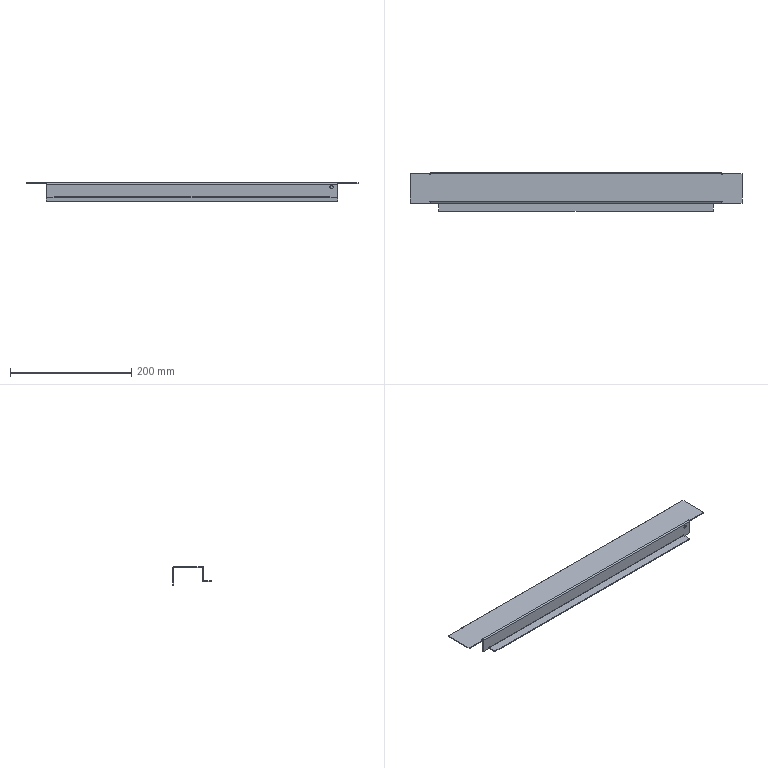Part | SolidWorks | features EdgeFlange 3, FlatPattern 1, ICE 1, SMBaseFlange 1, SheetMetal 1 | 1 solid | 56 faces | box 547 x 63.5 x 30 mm | volume 85940 mm3 | plane 48 | cylinder 8 | commonest cylinder face diameters 1 x3 4 x3 5.5 x2
STEP:
#1=CARTESIAN_POINT('',(230.,-22.75,-4.25));
#2=VERTEX_POINT('',#1);
#3=CARTESIAN_POINT('',(230.,-22.75,-9.75));
#4=VERTEX_POINT('',#3);
#5=CARTESIAN_POINT('',(230.,-22.75,-7.));
#6=DIRECTION('',(0.,-1.,0.));
#7=DIRECTION('',(0.,0.,-1.));
#8=AXIS2_PLACEMENT_3D('',#5,#6,#7);
#9=CIRCLE('',#8,2.75);
#10=EDGE_CURVE('',#2,#4,#9,.T.);
#11=ORIENTED_EDGE('',*,*,#10,.F.);
#12=CARTESIAN_POINT('',(230.,-24.25,-4.25));
#13=VERTEX_POINT('',#12);
#14=CARTESIAN_POINT('',(230.,-22.75,-4.25));
#15=DIRECTION('',(0.,-1.,0.));
#16=VECTOR('',#15,1000.);
#17=LINE('',#14,#16);
#18=EDGE_CURVE('',#2,#13,#17,.T.);
#19=ORIENTED_EDGE('',*,*,#18,.T.);
#20=CARTESIAN_POINT('',(230.,-24.25,-9.75));
#21=VERTEX_POINT('',#20);
#22=CARTESIAN_POINT('',(230.,-24.25,-7.));
#23=DIRECTION('',(0.,-1.,0.));
#24=DIRECTION('',(0.,0.,-1.));
#25=AXIS2_PLACEMENT_3D('',#22,#23,#24);
#26=CIRCLE('',#25,2.75);
#27=EDGE_CURVE('',#13,#21,#26,.T.);
#28=ORIENTED_EDGE('',*,*,#27,.T.);
#29=CARTESIAN_POINT('',(230.,-22.75,-9.75));
#30=DIRECTION('',(0.,-1.,0.));
#31=VECTOR('',#30,1000.);
#32=LINE('',#29,#31);
#33=EDGE_CURVE('',#4,#21,#32,.T.);
#34=ORIENTED_EDGE('',*,*,#33,.F.);
#35=EDGE_LOOP('',(#11,#19,#28,#34));
#36=FACE_OUTER_BOUND('',#35,.T.);
#37=CARTESIAN_POINT('',(230.,-22.75,-7.));
#38=DIRECTION('',(0.,-1.,0.));
#39=DIRECTION('',(0.,0.,-1.));
#40=AXIS2_PLACEMENT_3D('',#37,#38,#39);
#41=CYLINDRICAL_SURFACE('',#40,2.75);
#42=ADVANCED_FACE('',(#36),#41,.F.);
#43=CARTESIAN_POINT('',(240.75,24.25,-1.5));
#44=VERTEX_POINT('',#43);
#45=CARTESIAN_POINT('',(240.75,23.,-1.5));
#46=VERTEX_POINT('',#45);
#47=CARTESIAN_POINT('',(240.75,24.25,-1.5));
#48=DIRECTION('',(0.,-1.,0.));
#49=VECTOR('',#48,1000.);
#50=LINE('',#47,#49);
#51=EDGE_CURVE('',#44,#46,#50,.T.);
#52=ORIENTED_EDGE('',*,*,#51,.F.);
#53=CARTESIAN_POINT('',(273.5,24.25,-1.5));
#54=VERTEX_POINT('',#53);
#55=CARTESIAN_POINT('',(-273.5,24.25,-1.5));
#56=DIRECTION('',(-1.,0.,0.));
#57=VECTOR('',#56,1000.);
#58=LINE('',#55,#57);
#59=EDGE_CURVE('',#54,#44,#58,.T.);
#60=ORIENTED_EDGE('',*,*,#59,.F.);
#61=CARTESIAN_POINT('',(273.5,-24.25,-1.5));
#62=VERTEX_POINT('',#61);
#63=CARTESIAN_POINT('',(273.5,24.25,-1.5));
#64=DIRECTION('',(0.,1.,0.));
#65=VECTOR('',#64,1000.);
#66=LINE('',#63,#65);
#67=EDGE_CURVE('',#62,#54,#66,.T.);
#68=ORIENTED_EDGE('',*,*,#67,.F.);
#69=CARTESIAN_POINT('',(240.75,-24.25,-1.5));
#70=VERTEX_POINT('',#69);
#71=CARTESIAN_POINT('',(-273.5,-24.25,-1.5));
#72=DIRECTION('',(1.,0.,0.));
#73=VECTOR('',#72,1000.);
#74=LINE('',#71,#73);
#75=EDGE_CURVE('',#70,#62,#74,.T.);
#76=ORIENTED_EDGE('',*,*,#75,.F.);
#77=CARTESIAN_POINT('',(240.75,-21.5,-1.5));
#78=VERTEX_POINT('',#77);
#79=CARTESIAN_POINT('',(240.75,-21.5,-1.5));
#80=DIRECTION('',(0.,-1.,0.));
#81=VECTOR('',#80,1000.);
#82=LINE('',#79,#81);
#83=EDGE_CURVE('',#78,#70,#82,.T.);
#84=ORIENTED_EDGE('',*,*,#83,.F.);
#85=CARTESIAN_POINT('',(240.,-21.5,-1.5));
#86=VERTEX_POINT('',#85);
#87=CARTESIAN_POINT('',(240.,-21.5,-1.5));
#88=DIRECTION('',(1.,0.,0.));
#89=VECTOR('',#88,1000.);
#90=LINE('',#87,#89);
#91=EDGE_CURVE('',#86,#78,#90,.T.);
#92=ORIENTED_EDGE('',*,*,#91,.F.);
#93=CARTESIAN_POINT('',(240.,-22.25,-1.5));
#94=VERTEX_POINT('',#93);
#95=CARTESIAN_POINT('',(240.,-22.25,-1.5));
#96=DIRECTION('',(0.,1.,0.));
#97=VECTOR('',#96,1000.);
#98=LINE('',#95,#97);
#99=EDGE_CURVE('',#94,#86,#98,.T.);
#100=ORIENTED_EDGE('',*,*,#99,.F.);
#101=CARTESIAN_POINT('',(-240.,-22.25,-1.5));
#102=VERTEX_POINT('',#101);
#103=CARTESIAN_POINT('',(-240.,-22.25,-1.5));
#104=DIRECTION('',(1.,0.,0.));
#105=VECTOR('',#104,1000.);
#106=LINE('',#103,#105);
#107=EDGE_CURVE('',#102,#94,#106,.T.);
#108=ORIENTED_EDGE('',*,*,#107,.F.);
#109=CARTESIAN_POINT('',(-240.,-21.5,-1.5));
#110=VERTEX_POINT('',#109);
#111=CARTESIAN_POINT('',(-240.,-21.5,-1.5));
#112=DIRECTION('',(0.,-1.,0.));
#113=VECTOR('',#112,1000.);
#114=LINE('',#111,#113);
#115=EDGE_CURVE('',#110,#102,#114,.T.);
#116=ORIENTED_EDGE('',*,*,#115,.F.);
#117=CARTESIAN_POINT('',(-240.75,-21.5,-1.5));
#118=VERTEX_POINT('',#117);
#119=CARTESIAN_POINT('',(-240.75,-21.5,-1.5));
#120=DIRECTION('',(1.,0.,0.));
#121=VECTOR('',#120,1000.);
#122=LINE('',#119,#121);
#123=EDGE_CURVE('',#118,#110,#122,.T.);
#124=ORIENTED_EDGE('',*,*,#123,.F.);
#125=CARTESIAN_POINT('',(-240.75,-24.25,-1.5));
#126=VERTEX_POINT('',#125);
#127=CARTESIAN_POINT('',(-240.75,-24.25,-1.5));
#128=DIRECTION('',(0.,1.,0.));
#129=VECTOR('',#128,1000.);
#130=LINE('',#127,#129);
#131=EDGE_CURVE('',#126,#118,#130,.T.);
#132=ORIENTED_EDGE('',*,*,#131,.F.);
#133=CARTESIAN_POINT('',(-273.5,-24.25,-1.5));
#134=VERTEX_POINT('',#133);
#135=CARTESIAN_POINT('',(-273.5,-24.25,-1.5));
#136=DIRECTION('',(1.,0.,0.));
#137=VECTOR('',#136,1000.);
#138=LINE('',#135,#137);
#139=EDGE_CURVE('',#134,#126,#138,.T.);
#140=ORIENTED_EDGE('',*,*,#139,.F.);
#141=CARTESIAN_POINT('',(-273.5,24.25,-1.5));
#142=VERTEX_POINT('',#141);
#143=CARTESIAN_POINT('',(-273.5,24.25,-1.5));
#144=DIRECTION('',(0.,-1.,0.));
#145=VECTOR('',#144,1000.);
#146=LINE('',#143,#145);
#147=EDGE_CURVE('',#142,#134,#146,.T.);
#148=ORIENTED_EDGE('',*,*,#147,.F.);
#149=CARTESIAN_POINT('',(-240.75,24.25,-1.5));
#150=VERTEX_POINT('',#149);
#151=CARTESIAN_POINT('',(-273.5,24.25,-1.5));
#152=DIRECTION('',(-1.,0.,0.));
#153=VECTOR('',#152,1000.);
#154=LINE('',#151,#153);
#155=EDGE_CURVE('',#150,#142,#154,.T.);
#156=ORIENTED_EDGE('',*,*,#155,.F.);
#157=CARTESIAN_POINT('',(-240.75,23.,-1.5));
#158=VERTEX_POINT('',#157);
#159=CARTESIAN_POINT('',(-240.75,23.,-1.5));
#160=DIRECTION('',(0.,1.,0.));
#161=VECTOR('',#160,1000.);
#162=LINE('',#159,#161);
#163=EDGE_CURVE('',#158,#150,#162,.T.);
#164=ORIENTED_EDGE('',*,*,#163,.F.);
#165=CARTESIAN_POINT('',(-240.,23.,-1.5));
#166=VERTEX_POINT('',#165);
#167=CARTESIAN_POINT('',(-240.,23.,-1.5));
#168=DIRECTION('',(-1.,0.,0.));
#169=VECTOR('',#168,1000.);
#170=LINE('',#167,#169);
#171=EDGE_CURVE('',#166,#158,#170,.T.);
#172=ORIENTED_EDGE('',*,*,#171,.F.);
#173=CARTESIAN_POINT('',(-240.,23.75,-1.5));
#174=VERTEX_POINT('',#173);
#175=CARTESIAN_POINT('',(-240.,23.75,-1.5));
#176=DIRECTION('',(0.,-1.,0.));
#177=VECTOR('',#176,1000.);
#178=LINE('',#175,#177);
#179=EDGE_CURVE('',#174,#166,#178,.T.);
#180=ORIENTED_EDGE('',*,*,#179,.F.);
#181=CARTESIAN_POINT('',(240.,23.75,-1.5));
#182=VERTEX_POINT('',#181);
#183=CARTESIAN_POINT('',(240.,23.75,-1.5));
#184=DIRECTION('',(-1.,0.,0.));
#185=VECTOR('',#184,1000.);
#186=LINE('',#183,#185);
#187=EDGE_CURVE('',#182,#174,#186,.T.);
#188=ORIENTED_EDGE('',*,*,#187,.F.);
#189=CARTESIAN_POINT('',(240.,23.,-1.5));
#190=VERTEX_POINT('',#189);
#191=CARTESIAN_POINT('',(240.,23.,-1.5));
#192=DIRECTION('',(0.,1.,0.));
#193=VECTOR('',#192,1000.);
#194=LINE('',#191,#193);
#195=EDGE_CURVE('',#190,#182,#194,.T.);
#196=ORIENTED_EDGE('',*,*,#195,.F.);
#197=CARTESIAN_POINT('',(240.75,23.,-1.5));
#198=DIRECTION('',(-1.,0.,0.));
#199=VECTOR('',#198,1000.);
#200=LINE('',#197,#199);
#201=EDGE_CURVE('',#46,#190,#200,.T.);
#202=ORIENTED_EDGE('',*,*,#201,.F.);
#203=EDGE_LOOP('',(#52,#60,#68,#76,#84,#92,#100,#108,#116,#124,#132,#140,#148,#156,#164,#172,#180,#188,#196,#202));
#204=FACE_OUTER_BOUND('',#203,.T.);
#205=CARTESIAN_POINT('',(0.,0.,-1.5));
#206=DIRECTION('',(0.,0.,1.));
#207=DIRECTION('',(1.,0.,0.));
#208=AXIS2_PLACEMENT_3D('',#205,#206,#207);
#209=PLANE('',#208);
#210=ADVANCED_FACE('',(#204),#209,.F.);
#211=CARTESIAN_POINT('',(273.5,24.25,0.));
#212=VERTEX_POINT('',#211);
#213=CARTESIAN_POINT('',(240.75,24.25,0.));
#214=VERTEX_POINT('',#213);
#215=CARTESIAN_POINT('',(-273.5,24.25,0.));
#216=DIRECTION('',(-1.,0.,0.));
#217=VECTOR('',#216,1000.);
#218=LINE('',#215,#217);
#219=EDGE_CURVE('',#212,#214,#218,.T.);
#220=ORIENTED_EDGE('',*,*,#219,.T.);
#221=CARTESIAN_POINT('',(240.75,23.,0.));
#222=VERTEX_POINT('',#221);
#223=CARTESIAN_POINT('',(240.75,0.,0.));
#224=DIRECTION('',(0.,-1.,0.));
#225=VECTOR('',#224,1000.);
#226=LINE('',#223,#225);
#227=EDGE_CURVE('',#214,#222,#226,.T.);
#228=ORIENTED_EDGE('',*,*,#227,.T.);
#229=CARTESIAN_POINT('',(240.,23.,0.));
#230=VERTEX_POINT('',#229);
#231=CARTESIAN_POINT('',(0.,23.,0.));
#232=DIRECTION('',(-1.,0.,0.));
#233=VECTOR('',#232,1000.);
#234=LINE('',#231,#233);
#235=EDGE_CURVE('',#222,#230,#234,.T.);
#236=ORIENTED_EDGE('',*,*,#235,.T.);
#237=CARTESIAN_POINT('',(240.,23.75,0.));
#238=VERTEX_POINT('',#237);
#239=CARTESIAN_POINT('',(240.,0.,0.));
#240=DIRECTION('',(0.,1.,0.));
#241=VECTOR('',#240,1000.);
#242=LINE('',#239,#241);
#243=EDGE_CURVE('',#230,#238,#242,.T.);
#244=ORIENTED_EDGE('',*,*,#243,.T.);
#245=CARTESIAN_POINT('',(-240.,23.75,0.));
#246=VERTEX_POINT('',#245);
#247=CARTESIAN_POINT('',(240.,23.75,0.));
#248=DIRECTION('',(-1.,0.,0.));
#249=VECTOR('',#248,1000.);
#250=LINE('',#247,#249);
#251=EDGE_CURVE('',#238,#246,#250,.T.);
#252=ORIENTED_EDGE('',*,*,#251,.T.);
#253=CARTESIAN_POINT('',(-240.,23.,0.));
#254=VERTEX_POINT('',#253);
#255=CARTESIAN_POINT('',(-240.,0.,0.));
#256=DIRECTION('',(0.,-1.,0.));
#257=VECTOR('',#256,1000.);
#258=LINE('',#255,#257);
#259=EDGE_CURVE('',#246,#254,#258,.T.);
#260=ORIENTED_EDGE('',*,*,#259,.T.);
#261=CARTESIAN_POINT('',(-240.75,23.,0.));
#262=VERTEX_POINT('',#261);
#263=CARTESIAN_POINT('',(0.,23.,0.));
#264=DIRECTION('',(-1.,0.,0.));
#265=VECTOR('',#264,1000.);
#266=LINE('',#263,#265);
#267=EDGE_CURVE('',#254,#262,#266,.T.);
#268=ORIENTED_EDGE('',*,*,#267,.T.);
#269=CARTESIAN_POINT('',(-240.75,24.25,0.));
#270=VERTEX_POINT('',#269);
#271=CARTESIAN_POINT('',(-240.75,0.,0.));
#272=DIRECTION('',(0.,1.,0.));
#273=VECTOR('',#272,1000.);
#274=LINE('',#271,#273);
#275=EDGE_CURVE('',#262,#270,#274,.T.);
#276=ORIENTED_EDGE('',*,*,#275,.T.);
#277=CARTESIAN_POINT('',(-273.5,24.25,0.));
#278=VERTEX_POINT('',#277);
#279=CARTESIAN_POINT('',(-273.5,24.25,0.));
#280=DIRECTION('',(-1.,0.,0.));
#281=VECTOR('',#280,1000.);
#282=LINE('',#279,#281);
#283=EDGE_CURVE('',#270,#278,#282,.T.);
#284=ORIENTED_EDGE('',*,*,#283,.T.);
#285=CARTESIAN_POINT('',(-273.5,-24.25,0.));
#286=VERTEX_POINT('',#285);
#287=CARTESIAN_POINT('',(-273.5,24.25,0.));
#288=DIRECTION('',(0.,-1.,0.));
#289=VECTOR('',#288,1000.);
#290=LINE('',#287,#289);
#291=EDGE_CURVE('',#278,#286,#290,.T.);
#292=ORIENTED_EDGE('',*,*,#291,.T.);
#293=CARTESIAN_POINT('',(-240.75,-24.25,0.));
#294=VERTEX_POINT('',#293);
#295=CARTESIAN_POINT('',(-273.5,-24.25,0.));
#296=DIRECTION('',(1.,0.,0.));
#297=VECTOR('',#296,1000.);
#298=LINE('',#295,#297);
#299=EDGE_CURVE('',#286,#294,#298,.T.);
#300=ORIENTED_EDGE('',*,*,#299,.T.);
#301=CARTESIAN_POINT('',(-240.75,-21.5,0.));
#302=VERTEX_POINT('',#301);
#303=CARTESIAN_POINT('',(-240.75,0.,0.));
#304=DIRECTION('',(0.,1.,0.));
#305=VECTOR('',#304,1000.);
#306=LINE('',#303,#305);
#307=EDGE_CURVE('',#294,#302,#306,.T.);
#308=ORIENTED_EDGE('',*,*,#307,.T.);
#309=CARTESIAN_POINT('',(-240.,-21.5,0.));
#310=VERTEX_POINT('',#309);
#311=CARTESIAN_POINT('',(0.,-21.5,0.));
#312=DIRECTION('',(1.,0.,0.));
#313=VECTOR('',#312,1000.);
#314=LINE('',#311,#313);
#315=EDGE_CURVE('',#302,#310,#314,.T.);
#316=ORIENTED_EDGE('',*,*,#315,.T.);
#317=CARTESIAN_POINT('',(-240.,-22.25,0.));
#318=VERTEX_POINT('',#317);
#319=CARTESIAN_POINT('',(-240.,0.,0.));
#320=DIRECTION('',(0.,-1.,0.));
#321=VECTOR('',#320,1000.);
#322=LINE('',#319,#321);
#323=EDGE_CURVE('',#310,#318,#322,.T.);
#324=ORIENTED_EDGE('',*,*,#323,.T.);
#325=CARTESIAN_POINT('',(240.,-22.25,0.));
#326=VERTEX_POINT('',#325);
#327=CARTESIAN_POINT('',(-240.,-22.25,0.));
#328=DIRECTION('',(1.,0.,0.));
#329=VECTOR('',#328,1000.);
#330=LINE('',#327,#329);
#331=EDGE_CURVE('',#318,#326,#330,.T.);
#332=ORIENTED_EDGE('',*,*,#331,.T.);
#333=CARTESIAN_POINT('',(240.,-21.5,0.));
#334=VERTEX_POINT('',#333);
#335=CARTESIAN_POINT('',(240.,0.,0.));
#336=DIRECTION('',(0.,1.,0.));
#337=VECTOR('',#336,1000.);
#338=LINE('',#335,#337);
#339=EDGE_CURVE('',#326,#334,#338,.T.);
#340=ORIENTED_EDGE('',*,*,#339,.T.);
#341=CARTESIAN_POINT('',(240.75,-21.5,0.));
#342=VERTEX_POINT('',#341);
#343=CARTESIAN_POINT('',(0.,-21.5,0.));
#344=DIRECTION('',(1.,0.,0.));
#345=VECTOR('',#344,1000.);
#346=LINE('',#343,#345);
#347=EDGE_CURVE('',#334,#342,#346,.T.);
#348=ORIENTED_EDGE('',*,*,#347,.T.);
#349=CARTESIAN_POINT('',(240.75,-24.25,0.));
#350=VERTEX_POINT('',#349);
#351=CARTESIAN_POINT('',(240.75,0.,0.));
#352=DIRECTION('',(0.,-1.,0.));
#353=VECTOR('',#352,1000.);
#354=LINE('',#351,#353);
#355=EDGE_CURVE('',#342,#350,#354,.T.);
#356=ORIENTED_EDGE('',*,*,#355,.T.);
#357=CARTESIAN_POINT('',(273.5,-24.25,0.));
#358=VERTEX_POINT('',#357);
#359=CARTESIAN_POINT('',(-273.5,-24.25,0.));
#360=DIRECTION('',(1.,0.,0.));
#361=VECTOR('',#360,1000.);
#362=LINE('',#359,#361);
#363=EDGE_CURVE('',#350,#358,#362,.T.);
#364=ORIENTED_EDGE('',*,*,#363,.T.);
#365=CARTESIAN_POINT('',(273.5,24.25,0.));
#366=DIRECTION('',(0.,1.,0.));
#367=VECTOR('',#366,1000.);
#368=LINE('',#365,#367);
#369=EDGE_CURVE('',#358,#212,#368,.T.);
#370=ORIENTED_EDGE('',*,*,#369,.T.);
#371=EDGE_LOOP('',(#220,#228,#236,#244,#252,#260,#268,#276,#284,#292,#300,#308,#316,#324,#332,#340,#348,#356,#364,#370));
#372=FACE_OUTER_BOUND('',#371,.T.);
#373=CARTESIAN_POINT('',(0.,0.,0.));
#374=DIRECTION('',(0.,0.,1.));
#375=DIRECTION('',(1.,0.,0.));
#376=AXIS2_PLACEMENT_3D('',#373,#374,#375);
#377=PLANE('',#376);
#378=ADVANCED_FACE('',(#372),#377,.T.);
#379=ORIENTED_EDGE('',*,*,#59,.T.);
#380=CARTESIAN_POINT('',(240.75,24.25,-1.5));
#381=DIRECTION('',(0.,0.,1.));
#382=VECTOR('',#381,1000.);
#383=LINE('',#380,#382);
#384=EDGE_CURVE('',#44,#214,#383,.T.);
#385=ORIENTED_EDGE('',*,*,#384,.T.);
#386=ORIENTED_EDGE('',*,*,#219,.F.);
#387=CARTESIAN_POINT('',(273.5,24.25,-1.5));
#388=DIRECTION('',(0.,0.,1.));
#389=VECTOR('',#388,1000.);
#390=LINE('',#387,#389);
#391=EDGE_CURVE('',#54,#212,#390,.T.);
#392=ORIENTED_EDGE('',*,*,#391,.F.);
#393=EDGE_LOOP('',(#379,#385,#386,#392));
#394=FACE_OUTER_BOUND('',#393,.T.);
#395=CARTESIAN_POINT('',(-273.5,24.25,-1.5));
#396=DIRECTION('',(0.,1.,0.));
#397=DIRECTION('',(0.,0.,1.));
#398=AXIS2_PLACEMENT_3D('',#395,#396,#397);
#399=PLANE('',#398);
#400=ADVANCED_FACE('',(#394),#399,.T.);
#401=ORIENTED_EDGE('',*,*,#283,.F.);
#402=CARTESIAN_POINT('',(-240.75,24.25,-1.5));
#403=DIRECTION('',(0.,0.,1.));
#404=VECTOR('',#403,1000.);
#405=LINE('',#402,#404);
#406=EDGE_CURVE('',#150,#270,#405,.T.);
#407=ORIENTED_EDGE('',*,*,#406,.F.);
#408=ORIENTED_EDGE('',*,*,#155,.T.);
#409=CARTESIAN_POINT('',(-273.5,24.25,-1.5));
#410=DIRECTION('',(0.,0.,1.));
#411=VECTOR('',#410,1000.);
#412=LINE('',#409,#411);
#413=EDGE_CURVE('',#142,#278,#412,.T.);
#414=ORIENTED_EDGE('',*,*,#413,.T.);
#415=EDGE_LOOP('',(#401,#407,#408,#414));
#416=FACE_OUTER_BOUND('',#415,.T.);
#417=CARTESIAN_POINT('',(-273.5,24.25,-1.5));
#418=DIRECTION('',(0.,1.,0.));
#419=DIRECTION('',(0.,0.,1.));
#420=AXIS2_PLACEMENT_3D('',#417,#418,#419);
#421=PLANE('',#420);
#422=ADVANCED_FACE('',(#416),#421,.T.);
#423=CARTESIAN_POINT('',(230.,-24.25,-7.));
#424=DIRECTION('',(0.,-1.,0.));
#425=DIRECTION('',(0.,0.,-1.));
#426=AXIS2_PLACEMENT_3D('',#423,#424,#425);
#427=CIRCLE('',#426,2.75);
#428=EDGE_CURVE('',#21,#13,#427,.T.);
#429=ORIENTED_EDGE('',*,*,#428,.F.);
#430=ORIENTED_EDGE('',*,*,#27,.F.);
#431=EDGE_LOOP('',(#429,#430));
#432=FACE_BOUND('',#431,.T.);
#433=CARTESIAN_POINT('',(227.25,-24.25,-21.75));
#434=VERTEX_POINT('',#433);
#435=CARTESIAN_POINT('',(226.5,-24.25,-21.75));
#436=VERTEX_POINT('',#435);
#437=CARTESIAN_POINT('',(227.25,-24.25,-21.75));
#438=DIRECTION('',(-1.,0.,0.));
#439=VECTOR('',#438,1000.);
#440=LINE('',#437,#439);
#441=EDGE_CURVE('',#434,#436,#440,.T.);
#442=ORIENTED_EDGE('',*,*,#441,.F.);
#443=CARTESIAN_POINT('',(227.25,-24.25,-24.5));
#444=VERTEX_POINT('',#443);
#445=CARTESIAN_POINT('',(227.25,-24.25,-24.5));
#446=DIRECTION('',(0.,0.,1.));
#447=VECTOR('',#446,1000.);
#448=LINE('',#445,#447);
#449=EDGE_CURVE('',#444,#434,#448,.T.);
#450=ORIENTED_EDGE('',*,*,#449,.F.);
#451=CARTESIAN_POINT('',(240.,-24.25,-24.5));
#452=VERTEX_POINT('',#451);
#453=CARTESIAN_POINT('',(-240.,-24.25,-24.5));
#454=DIRECTION('',(-1.,0.,0.));
#455=VECTOR('',#454,1000.);
#456=LINE('',#453,#455);
#457=EDGE_CURVE('',#452,#444,#456,.T.);
#458=ORIENTED_EDGE('',*,*,#457,.F.);
#459=CARTESIAN_POINT('',(240.,-24.25,-2.));
#460=VERTEX_POINT('',#459);
#461=CARTESIAN_POINT('',(240.,-24.25,-24.5));
#462=DIRECTION('',(0.,0.,-1.));
#463=VECTOR('',#462,1000.);
#464=LINE('',#461,#463);
#465=EDGE_CURVE('',#460,#452,#464,.T.);
#466=ORIENTED_EDGE('',*,*,#465,.F.);
#467=CARTESIAN_POINT('',(-240.,-24.25,-2.));
#468=VERTEX_POINT('',#467);
#469=CARTESIAN_POINT('',(0.,-24.25,-2.));
#470=DIRECTION('',(-1.,0.,0.));
#471=VECTOR('',#470,1000.);
#472=LINE('',#469,#471);
#473=EDGE_CURVE('',#460,#468,#472,.T.);
#474=ORIENTED_EDGE('',*,*,#473,.T.);
#475=CARTESIAN_POINT('',(-240.,-24.25,-24.5));
#476=VERTEX_POINT('',#475);
#477=CARTESIAN_POINT('',(-240.,-24.25,-1.5));
#478=DIRECTION('',(0.,0.,1.));
#479=VECTOR('',#478,1000.);
#480=LINE('',#477,#479);
#481=EDGE_CURVE('',#476,#468,#480,.T.);
#482=ORIENTED_EDGE('',*,*,#481,.F.);
#483=CARTESIAN_POINT('',(-227.25,-24.25,-24.5));
#484=VERTEX_POINT('',#483);
#485=CARTESIAN_POINT('',(-240.,-24.25,-24.5));
#486=DIRECTION('',(-1.,0.,0.));
#487=VECTOR('',#486,1000.);
#488=LINE('',#485,#487);
#489=EDGE_CURVE('',#484,#476,#488,.T.);
#490=ORIENTED_EDGE('',*,*,#489,.F.);
#491=CARTESIAN_POINT('',(-227.25,-24.25,-21.75));
#492=VERTEX_POINT('',#491);
#493=CARTESIAN_POINT('',(-227.25,-24.25,-21.75));
#494=DIRECTION('',(0.,0.,-1.));
#495=VECTOR('',#494,1000.);
#496=LINE('',#493,#495);
#497=EDGE_CURVE('',#492,#484,#496,.T.);
#498=ORIENTED_EDGE('',*,*,#497,.F.);
#499=CARTESIAN_POINT('',(-226.5,-24.25,-21.75));
#500=VERTEX_POINT('',#499);
#501=CARTESIAN_POINT('',(-226.5,-24.25,-21.75));
#502=DIRECTION('',(-1.,0.,0.));
#503=VECTOR('',#502,1000.);
#504=LINE('',#501,#503);
#505=EDGE_CURVE('',#500,#492,#504,.T.);
#506=ORIENTED_EDGE('',*,*,#505,.F.);
#507=CARTESIAN_POINT('',(-226.5,-24.25,-22.5));
#508=VERTEX_POINT('',#507);
#509=CARTESIAN_POINT('',(-226.5,-24.25,-22.5));
#510=DIRECTION('',(0.,0.,1.));
#511=VECTOR('',#510,1000.);
#512=LINE('',#509,#511);
#513=EDGE_CURVE('',#508,#500,#512,.T.);
#514=ORIENTED_EDGE('',*,*,#513,.F.);
#515=CARTESIAN_POINT('',(226.5,-24.25,-22.5));
#516=VERTEX_POINT('',#515);
#517=CARTESIAN_POINT('',(226.5,-24.25,-22.5));
#518=DIRECTION('',(-1.,0.,0.));
#519=VECTOR('',#518,1000.);
#520=LINE('',#517,#519);
#521=EDGE_CURVE('',#516,#508,#520,.T.);
#522=ORIENTED_EDGE('',*,*,#521,.F.);
#523=CARTESIAN_POINT('',(226.5,-24.25,-21.75));
#524=DIRECTION('',(0.,0.,-1.));
#525=VECTOR('',#524,1000.);
#526=LINE('',#523,#525);
#527=EDGE_CURVE('',#436,#516,#526,.T.);
#528=ORIENTED_EDGE('',*,*,#527,.F.);
#529=EDGE_LOOP('',(#442,#450,#458,#466,#474,#482,#490,#498,#506,#514,#522,#528));
#530=FACE_OUTER_BOUND('',#529,.T.);
#531=CARTESIAN_POINT('',(0.,-24.25,0.));
#532=DIRECTION('',(0.,-1.,0.));
#533=DIRECTION('',(0.,0.,-1.));
#534=AXIS2_PLACEMENT_3D('',#531,#532,#533);
#535=PLANE('',#534);
#536=ADVANCED_FACE('',(#432,#530),#535,.T.);
#537=CARTESIAN_POINT('',(230.,-22.75,-7.));
#538=DIRECTION('',(0.,-1.,0.));
#539=DIRECTION('',(0.,0.,-1.));
#540=AXIS2_PLACEMENT_3D('',#537,#538,#539);
#541=CIRCLE('',#540,2.75);
#542=EDGE_CURVE('',#4,#2,#541,.T.);
#543=ORIENTED_EDGE('',*,*,#542,.T.);
#544=ORIENTED_EDGE('',*,*,#10,.T.);
#545=EDGE_LOOP('',(#543,#544));
#546=FACE_BOUND('',#545,.T.);
#547=CARTESIAN_POINT('',(227.25,-22.75,-21.75));
#548=VERTEX_POINT('',#547);
#549=CARTESIAN_POINT('',(227.25,-22.75,-24.5));
#550=VERTEX_POINT('',#549);
#551=CARTESIAN_POINT('',(227.25,-22.75,0.));
#552=DIRECTION('',(0.,0.,-1.));
#553=VECTOR('',#552,1000.);
#554=LINE('',#551,#553);
#555=EDGE_CURVE('',#548,#550,#554,.T.);
#556=ORIENTED_EDGE('',*,*,#555,.F.);
#557=CARTESIAN_POINT('',(226.5,-22.75,-21.75));
#558=VERTEX_POINT('',#557);
#559=CARTESIAN_POINT('',(0.,-22.75,-21.75));
#560=DIRECTION('',(1.,0.,0.));
#561=VECTOR('',#560,1000.);
#562=LINE('',#559,#561);
#563=EDGE_CURVE('',#558,#548,#562,.T.);
#564=ORIENTED_EDGE('',*,*,#563,.F.);
#565=CARTESIAN_POINT('',(226.5,-22.75,-22.5));
#566=VERTEX_POINT('',#565);
#567=CARTESIAN_POINT('',(226.5,-22.75,0.));
#568=DIRECTION('',(0.,0.,1.));
#569=VECTOR('',#568,1000.);
#570=LINE('',#567,#569);
#571=EDGE_CURVE('',#566,#558,#570,.T.);
#572=ORIENTED_EDGE('',*,*,#571,.F.);
#573=CARTESIAN_POINT('',(-226.5,-22.75,-22.5));
#574=VERTEX_POINT('',#573);
#575=CARTESIAN_POINT('',(226.5,-22.75,-22.5));
#576=DIRECTION('',(-1.,0.,0.));
#577=VECTOR('',#576,1000.);
#578=LINE('',#575,#577);
#579=EDGE_CURVE('',#566,#574,#578,.T.);
#580=ORIENTED_EDGE('',*,*,#579,.T.);
#581=CARTESIAN_POINT('',(-226.5,-22.75,-21.75));
#582=VERTEX_POINT('',#581);
#583=CARTESIAN_POINT('',(-226.5,-22.75,0.));
#584=DIRECTION('',(0.,0.,-1.));
#585=VECTOR('',#584,1000.);
#586=LINE('',#583,#585);
#587=EDGE_CURVE('',#582,#574,#586,.T.);
#588=ORIENTED_EDGE('',*,*,#587,.F.);
#589=CARTESIAN_POINT('',(-227.25,-22.75,-21.75));
#590=VERTEX_POINT('',#589);
#591=CARTESIAN_POINT('',(0.,-22.75,-21.75));
#592=DIRECTION('',(1.,0.,0.));
#593=VECTOR('',#592,1000.);
#594=LINE('',#591,#593);
#595=EDGE_CURVE('',#590,#582,#594,.T.);
#596=ORIENTED_EDGE('',*,*,#595,.F.);
#597=CARTESIAN_POINT('',(-227.25,-22.75,-24.5));
#598=VERTEX_POINT('',#597);
#599=CARTESIAN_POINT('',(-227.25,-22.75,0.));
#600=DIRECTION('',(0.,0.,1.));
#601=VECTOR('',#600,1000.);
#602=LINE('',#599,#601);
#603=EDGE_CURVE('',#598,#590,#602,.T.);
#604=ORIENTED_EDGE('',*,*,#603,.F.);
#605=CARTESIAN_POINT('',(-240.,-22.75,-24.5));
#606=VERTEX_POINT('',#605);
#607=CARTESIAN_POINT('',(0.,-22.75,-24.5));
#608=DIRECTION('',(-1.,0.,0.));
#609=VECTOR('',#608,1000.);
#610=LINE('',#607,#609);
#611=EDGE_CURVE('',#598,#606,#610,.T.);
#612=ORIENTED_EDGE('',*,*,#611,.T.);
#613=CARTESIAN_POINT('',(-240.,-22.75,-2.));
#614=VERTEX_POINT('',#613);
#615=CARTESIAN_POINT('',(-240.,-22.75,0.));
#616=DIRECTION('',(0.,0.,1.));
#617=VECTOR('',#616,1000.);
#618=LINE('',#615,#617);
#619=EDGE_CURVE('',#606,#614,#618,.T.);
#620=ORIENTED_EDGE('',*,*,#619,.T.);
#621=CARTESIAN_POINT('',(240.,-22.75,-2.));
#622=VERTEX_POINT('',#621);
#623=CARTESIAN_POINT('',(240.,-22.75,-2.));
#624=DIRECTION('',(-1.,0.,0.));
#625=VECTOR('',#624,1000.);
#626=LINE('',#623,#625);
#627=EDGE_CURVE('',#622,#614,#626,.T.);
#628=ORIENTED_EDGE('',*,*,#627,.F.);
#629=CARTESIAN_POINT('',(240.,-22.75,-24.5));
#630=VERTEX_POINT('',#629);
#631=CARTESIAN_POINT('',(240.,-22.75,0.));
#632=DIRECTION('',(0.,0.,-1.));
#633=VECTOR('',#632,1000.);
#634=LINE('',#631,#633);
#635=EDGE_CURVE('',#622,#630,#634,.T.);
#636=ORIENTED_EDGE('',*,*,#635,.T.);
#637=CARTESIAN_POINT('',(0.,-22.75,-24.5));
#638=DIRECTION('',(-1.,0.,0.));
#639=VECTOR('',#638,1000.);
#640=LINE('',#637,#639);
#641=EDGE_CURVE('',#630,#550,#640,.T.);
#642=ORIENTED_EDGE('',*,*,#641,.T.);
#643=EDGE_LOOP('',(#556,#564,#572,#580,#588,#596,#604,#612,#620,#628,#636,#642));
#644=FACE_OUTER_BOUND('',#643,.T.);
#645=CARTESIAN_POINT('',(0.,-22.75,0.));
#646=DIRECTION('',(0.,-1.,0.));
#647=DIRECTION('',(0.,0.,-1.));
#648=AXIS2_PLACEMENT_3D('',#645,#646,#647);
#649=PLANE('',#648);
#650=ADVANCED_FACE('',(#546,#644),#649,.F.);
#651=ORIENTED_EDGE('',*,*,#457,.T.);
#652=CARTESIAN_POINT('',(227.25,-24.25,-24.5));
#653=DIRECTION('',(0.,1.,0.));
#654=VECTOR('',#653,1000.);
#655=LINE('',#652,#654);
#656=EDGE_CURVE('',#444,#550,#655,.T.);
#657=ORIENTED_EDGE('',*,*,#656,.T.);
#658=ORIENTED_EDGE('',*,*,#641,.F.);
#659=CARTESIAN_POINT('',(240.,-24.25,-24.5));
#660=DIRECTION('',(0.,1.,0.));
#661=VECTOR('',#660,1000.);
#662=LINE('',#659,#661);
#663=EDGE_CURVE('',#452,#630,#662,.T.);
#664=ORIENTED_EDGE('',*,*,#663,.F.);
#665=EDGE_LOOP('',(#651,#657,#658,#664));
#666=FACE_OUTER_BOUND('',#665,.T.);
#667=CARTESIAN_POINT('',(-240.,-24.25,-24.5));
#668=DIRECTION('',(0.,0.,-1.));
#669=DIRECTION('',(0.,1.,0.));
#670=AXIS2_PLACEMENT_3D('',#667,#668,#669);
#671=PLANE('',#670);
#672=ADVANCED_FACE('',(#666),#671,.T.);
#673=ORIENTED_EDGE('',*,*,#611,.F.);
#674=CARTESIAN_POINT('',(-227.25,-24.25,-24.5));
#675=DIRECTION('',(0.,1.,0.));
#676=VECTOR('',#675,1000.);
#677=LINE('',#674,#676);
#678=EDGE_CURVE('',#484,#598,#677,.T.);
#679=ORIENTED_EDGE('',*,*,#678,.F.);
#680=ORIENTED_EDGE('',*,*,#489,.T.);
#681=CARTESIAN_POINT('',(-240.,-24.25,-24.5));
#682=DIRECTION('',(0.,1.,0.));
#683=VECTOR('',#682,1000.);
#684=LINE('',#681,#683);
#685=EDGE_CURVE('',#476,#606,#684,.T.);
#686=ORIENTED_EDGE('',*,*,#685,.T.);
#687=EDGE_LOOP('',(#673,#679,#680,#686));
#688=FACE_OUTER_BOUND('',#687,.T.);
#689=CARTESIAN_POINT('',(-240.,-24.25,-24.5));
#690=DIRECTION('',(0.,0.,-1.));
#691=DIRECTION('',(0.,1.,0.));
#692=AXIS2_PLACEMENT_3D('',#689,#690,#691);
#693=PLANE('',#692);
#694=ADVANCED_FACE('',(#688),#693,.T.);
#695=ORIENTED_EDGE('',*,*,#139,.T.);
#696=CARTESIAN_POINT('',(-240.75,-24.25,-1.5));
#697=DIRECTION('',(0.,0.,1.));
#698=VECTOR('',#697,1000.);
#699=LINE('',#696,#698);
#700=EDGE_CURVE('',#126,#294,#699,.T.);
#701=ORIENTED_EDGE('',*,*,#700,.T.);
#702=ORIENTED_EDGE('',*,*,#299,.F.);
#703=CARTESIAN_POINT('',(-273.5,-24.25,-1.5));
#704=DIRECTION('',(0.,0.,1.));
#705=VECTOR('',#704,1000.);
#706=LINE('',#703,#705);
#707=EDGE_CURVE('',#134,#286,#706,.T.);
#708=ORIENTED_EDGE('',*,*,#707,.F.);
#709=EDGE_LOOP('',(#695,#701,#702,#708));
#710=FACE_OUTER_BOUND('',#709,.T.);
#711=CARTESIAN_POINT('',(-273.5,-24.25,-1.5));
#712=DIRECTION('',(0.,-1.,0.));
#713=DIRECTION('',(0.,0.,-1.));
#714=AXIS2_PLACEMENT_3D('',#711,#712,#713);
#715=PLANE('',#714);
#716=ADVANCED_FACE('',(#710),#715,.T.);
#717=ORIENTED_EDGE('',*,*,#363,.F.);
#718=CARTESIAN_POINT('',(240.75,-24.25,-1.5));
#719=DIRECTION('',(0.,0.,1.));
#720=VECTOR('',#719,1000.);
#721=LINE('',#718,#720);
#722=EDGE_CURVE('',#70,#350,#721,.T.);
#723=ORIENTED_EDGE('',*,*,#722,.F.);
#724=ORIENTED_EDGE('',*,*,#75,.T.);
#725=CARTESIAN_POINT('',(273.5,-24.25,-1.5));
#726=DIRECTION('',(0.,0.,1.));
#727=VECTOR('',#726,1000.);
#728=LINE('',#725,#727);
#729=EDGE_CURVE('',#62,#358,#728,.T.);
#730=ORIENTED_EDGE('',*,*,#729,.T.);
#731=EDGE_LOOP('',(#717,#723,#724,#730));
#732=FACE_OUTER_BOUND('',#731,.T.);
#733=CARTESIAN_POINT('',(-273.5,-24.25,-1.5));
#734=DIRECTION('',(0.,-1.,0.));
#735=DIRECTION('',(0.,0.,-1.));
#736=AXIS2_PLACEMENT_3D('',#733,#734,#735);
#737=PLANE('',#736);
#738=ADVANCED_FACE('',(#732),#737,.T.);
#739=ORIENTED_EDGE('',*,*,#369,.F.);
#740=ORIENTED_EDGE('',*,*,#729,.F.);
#741=ORIENTED_EDGE('',*,*,#67,.T.);
#742=ORIENTED_EDGE('',*,*,#391,.T.);
#743=EDGE_LOOP('',(#739,#740,#741,#742));
#744=FACE_OUTER_BOUND('',#743,.T.);
#745=CARTESIAN_POINT('',(273.5,24.25,-1.5));
#746=DIRECTION('',(1.,0.,0.));
#747=DIRECTION('',(0.,0.,-1.));
#748=AXIS2_PLACEMENT_3D('',#745,#746,#747);
#749=PLANE('',#748);
#750=ADVANCED_FACE('',(#744),#749,.T.);
#751=ORIENTED_EDGE('',*,*,#291,.F.);
#752=ORIENTED_EDGE('',*,*,#413,.F.);
#753=ORIENTED_EDGE('',*,*,#147,.T.);
#754=ORIENTED_EDGE('',*,*,#707,.T.);
#755=EDGE_LOOP('',(#751,#752,#753,#754));
#756=FACE_OUTER_BOUND('',#755,.T.);
#757=CARTESIAN_POINT('',(-273.5,24.25,-1.5));
#758=DIRECTION('',(-1.,0.,0.));
#759=DIRECTION('',(0.,0.,1.));
#760=AXIS2_PLACEMENT_3D('',#757,#758,#759);
#761=PLANE('',#760);
#762=ADVANCED_FACE('',(#756),#761,.T.);
#763=ORIENTED_EDGE('',*,*,#307,.F.);
#764=ORIENTED_EDGE('',*,*,#700,.F.);
#765=ORIENTED_EDGE('',*,*,#131,.T.);
#766=CARTESIAN_POINT('',(-240.75,-21.5,-1.5));
#767=DIRECTION('',(0.,0.,1.));
#768=VECTOR('',#767,1000.);
#769=LINE('',#766,#768);
#770=EDGE_CURVE('',#118,#302,#769,.T.);
#771=ORIENTED_EDGE('',*,*,#770,.T.);
#772=EDGE_LOOP('',(#763,#764,#765,#771));
#773=FACE_OUTER_BOUND('',#772,.T.);
#774=CARTESIAN_POINT('',(-240.75,-24.25,-1.5));
#775=DIRECTION('',(1.,0.,0.));
#776=DIRECTION('',(0.,0.,-1.));
#777=AXIS2_PLACEMENT_3D('',#774,#775,#776);
#778=PLANE('',#777);
#779=ADVANCED_FACE('',(#773),#778,.T.);
#780=ORIENTED_EDGE('',*,*,#315,.F.);
#781=ORIENTED_EDGE('',*,*,#770,.F.);
#782=ORIENTED_EDGE('',*,*,#123,.T.);
#783=CARTESIAN_POINT('',(-240.,-21.5,-1.5));
#784=DIRECTION('',(0.,0.,1.));
#785=VECTOR('',#784,1000.);
#786=LINE('',#783,#785);
#787=EDGE_CURVE('',#110,#310,#786,.T.);
#788=ORIENTED_EDGE('',*,*,#787,.T.);
#789=EDGE_LOOP('',(#780,#781,#782,#788));
#790=FACE_OUTER_BOUND('',#789,.T.);
#791=CARTESIAN_POINT('',(-240.75,-21.5,-1.5));
#792=DIRECTION('',(0.,-1.,0.));
#793=DIRECTION('',(0.,0.,-1.));
#794=AXIS2_PLACEMENT_3D('',#791,#792,#793);
#795=PLANE('',#794);
#796=ADVANCED_FACE('',(#790),#795,.T.);
#797=ORIENTED_EDGE('',*,*,#323,.F.);
#798=ORIENTED_EDGE('',*,*,#787,.F.);
#799=ORIENTED_EDGE('',*,*,#115,.T.);
#800=CARTESIAN_POINT('',(-240.,-22.25,-1.5));
#801=DIRECTION('',(0.,0.,1.));
#802=VECTOR('',#801,1000.);
#803=LINE('',#800,#802);
#804=EDGE_CURVE('',#102,#318,#803,.T.);
#805=ORIENTED_EDGE('',*,*,#804,.T.);
#806=EDGE_LOOP('',(#797,#798,#799,#805));
#807=FACE_OUTER_BOUND('',#806,.T.);
#808=CARTESIAN_POINT('',(-240.,-21.5,-1.5));
#809=DIRECTION('',(-1.,0.,0.));
#810=DIRECTION('',(0.,0.,1.));
#811=AXIS2_PLACEMENT_3D('',#808,#809,#810);
#812=PLANE('',#811);
#813=ADVANCED_FACE('',(#807),#812,.T.);
#814=ORIENTED_EDGE('',*,*,#339,.F.);
#815=CARTESIAN_POINT('',(240.,-22.25,-1.5));
#816=DIRECTION('',(0.,0.,1.));
#817=VECTOR('',#816,1000.);
#818=LINE('',#815,#817);
#819=EDGE_CURVE('',#94,#326,#818,.T.);
#820=ORIENTED_EDGE('',*,*,#819,.F.);
#821=ORIENTED_EDGE('',*,*,#99,.T.);
#822=CARTESIAN_POINT('',(240.,-21.5,-1.5));
#823=DIRECTION('',(0.,0.,1.));
#824=VECTOR('',#823,1000.);
#825=LINE('',#822,#824);
#826=EDGE_CURVE('',#86,#334,#825,.T.);
#827=ORIENTED_EDGE('',*,*,#826,.T.);
#828=EDGE_LOOP('',(#814,#820,#821,#827));
#829=FACE_OUTER_BOUND('',#828,.T.);
#830=CARTESIAN_POINT('',(240.,-22.25,-1.5));
#831=DIRECTION('',(1.,0.,0.));
#832=DIRECTION('',(0.,0.,-1.));
#833=AXIS2_PLACEMENT_3D('',#830,#831,#832);
#834=PLANE('',#833);
#835=ADVANCED_FACE('',(#829),#834,.T.);
#836=ORIENTED_EDGE('',*,*,#347,.F.);
#837=ORIENTED_EDGE('',*,*,#826,.F.);
#838=ORIENTED_EDGE('',*,*,#91,.T.);
#839=CARTESIAN_POINT('',(240.75,-21.5,-1.5));
#840=DIRECTION('',(0.,0.,1.));
#841=VECTOR('',#840,1000.);
#842=LINE('',#839,#841);
#843=EDGE_CURVE('',#78,#342,#842,.T.);
#844=ORIENTED_EDGE('',*,*,#843,.T.);
#845=EDGE_LOOP('',(#836,#837,#838,#844));
#846=FACE_OUTER_BOUND('',#845,.T.);
#847=CARTESIAN_POINT('',(240.,-21.5,-1.5));
#848=DIRECTION('',(0.,-1.,0.));
#849=DIRECTION('',(0.,0.,-1.));
#850=AXIS2_PLACEMENT_3D('',#847,#848,#849);
#851=PLANE('',#850);
#852=ADVANCED_FACE('',(#846),#851,.T.);
#853=ORIENTED_EDGE('',*,*,#355,.F.);
#854=ORIENTED_EDGE('',*,*,#843,.F.);
#855=ORIENTED_EDGE('',*,*,#83,.T.);
#856=ORIENTED_EDGE('',*,*,#722,.T.);
#857=EDGE_LOOP('',(#853,#854,#855,#856));
#858=FACE_OUTER_BOUND('',#857,.T.);
#859=CARTESIAN_POINT('',(240.75,-21.5,-1.5));
#860=DIRECTION('',(-1.,0.,0.));
#861=DIRECTION('',(0.,-1.,0.));
#862=AXIS2_PLACEMENT_3D('',#859,#860,#861);
#863=PLANE('',#862);
#864=ADVANCED_FACE('',(#858),#863,.T.);
#865=CARTESIAN_POINT('',(240.,-24.25,-2.));
#866=DIRECTION('',(0.,-1.,0.));
#867=VECTOR('',#866,1000.);
#868=LINE('',#865,#867);
#869=EDGE_CURVE('',#622,#460,#868,.T.);
#870=ORIENTED_EDGE('',*,*,#869,.F.);
#871=CARTESIAN_POINT('',(240.,-22.25,-2.));
#872=DIRECTION('',(1.,0.,0.));
#873=DIRECTION('',(0.,0.,1.));
#874=AXIS2_PLACEMENT_3D('',#871,#872,#873);
#875=CIRCLE('',#874,0.5);
#876=EDGE_CURVE('',#94,#622,#875,.T.);
#877=ORIENTED_EDGE('',*,*,#876,.F.);
#878=ORIENTED_EDGE('',*,*,#819,.T.);
#879=CARTESIAN_POINT('',(240.,-22.25,-2.));
#880=DIRECTION('',(1.,0.,0.));
#881=DIRECTION('',(0.,0.,1.));
#882=AXIS2_PLACEMENT_3D('',#879,#880,#881);
#883=CIRCLE('',#882,2.);
#884=EDGE_CURVE('',#326,#460,#883,.T.);
#885=ORIENTED_EDGE('',*,*,#884,.T.);
#886=EDGE_LOOP('',(#870,#877,#878,#885));
#887=FACE_OUTER_BOUND('',#886,.T.);
#888=CARTESIAN_POINT('',(240.,-22.25,-2.));
#889=DIRECTION('',(1.,0.,0.));
#890=DIRECTION('',(0.,0.,-1.));
#891=AXIS2_PLACEMENT_3D('',#888,#889,#890);
#892=PLANE('',#891);
#893=ADVANCED_FACE('',(#887),#892,.T.);
#894=CARTESIAN_POINT('',(-240.,-22.25,-2.));
#895=DIRECTION('',(-1.,0.,0.));
#896=DIRECTION('',(0.,0.,1.));
#897=AXIS2_PLACEMENT_3D('',#894,#895,#896);
#898=CIRCLE('',#897,0.5);
#899=EDGE_CURVE('',#614,#102,#898,.T.);
#900=ORIENTED_EDGE('',*,*,#899,.F.);
#901=CARTESIAN_POINT('',(-240.,-22.75,-2.));
#902=DIRECTION('',(0.,-1.,0.));
#903=VECTOR('',#902,1000.);
#904=LINE('',#901,#903);
#905=EDGE_CURVE('',#614,#468,#904,.T.);
#906=ORIENTED_EDGE('',*,*,#905,.T.);
#907=CARTESIAN_POINT('',(-240.,-22.25,-2.));
#908=DIRECTION('',(-1.,0.,0.));
#909=DIRECTION('',(0.,0.,1.));
#910=AXIS2_PLACEMENT_3D('',#907,#908,#909);
#911=CIRCLE('',#910,2.);
#912=EDGE_CURVE('',#468,#318,#911,.T.);
#913=ORIENTED_EDGE('',*,*,#912,.T.);
#914=ORIENTED_EDGE('',*,*,#804,.F.);
#915=EDGE_LOOP('',(#900,#906,#913,#914));
#916=FACE_OUTER_BOUND('',#915,.T.);
#917=CARTESIAN_POINT('',(-240.,-22.25,-2.));
#918=DIRECTION('',(1.,0.,0.));
#919=DIRECTION('',(0.,0.,-1.));
#920=AXIS2_PLACEMENT_3D('',#917,#918,#919);
#921=PLANE('',#920);
#922=ADVANCED_FACE('',(#916),#921,.F.);
#923=ORIENTED_EDGE('',*,*,#331,.F.);
#924=ORIENTED_EDGE('',*,*,#912,.F.);
#925=ORIENTED_EDGE('',*,*,#473,.F.);
#926=ORIENTED_EDGE('',*,*,#884,.F.);
#927=EDGE_LOOP('',(#923,#924,#925,#926));
#928=FACE_OUTER_BOUND('',#927,.T.);
#929=CARTESIAN_POINT('',(-240.,-22.25,-2.));
#930=DIRECTION('',(-1.,0.,0.));
#931=DIRECTION('',(0.,-1.,0.));
#932=AXIS2_PLACEMENT_3D('',#929,#930,#931);
#933=CYLINDRICAL_SURFACE('',#932,2.);
#934=ADVANCED_FACE('',(#928),#933,.T.);
#935=ORIENTED_EDGE('',*,*,#107,.T.);
#936=ORIENTED_EDGE('',*,*,#876,.T.);
#937=ORIENTED_EDGE('',*,*,#627,.T.);
#938=ORIENTED_EDGE('',*,*,#899,.T.);
#939=EDGE_LOOP('',(#935,#936,#937,#938));
#940=FACE_OUTER_BOUND('',#939,.T.);
#941=CARTESIAN_POINT('',(-240.,-22.25,-2.));
#942=DIRECTION('',(-1.,0.,0.));
#943=DIRECTION('',(0.,-1.,0.));
#944=AXIS2_PLACEMENT_3D('',#941,#942,#943);
#945=CYLINDRICAL_SURFACE('',#944,0.5);
#946=ADVANCED_FACE('',(#940),#945,.F.);
#947=ORIENTED_EDGE('',*,*,#481,.T.);
#948=ORIENTED_EDGE('',*,*,#905,.F.);
#949=ORIENTED_EDGE('',*,*,#619,.F.);
#950=ORIENTED_EDGE('',*,*,#685,.F.);
#951=EDGE_LOOP('',(#947,#948,#949,#950));
#952=FACE_OUTER_BOUND('',#951,.T.);
#953=CARTESIAN_POINT('',(-240.,-24.25,-1.5));
#954=DIRECTION('',(-1.,0.,0.));
#955=DIRECTION('',(0.,0.,1.));
#956=AXIS2_PLACEMENT_3D('',#953,#954,#955);
#957=PLANE('',#956);
#958=ADVANCED_FACE('',(#952),#957,.T.);
#959=ORIENTED_EDGE('',*,*,#635,.F.);
#960=ORIENTED_EDGE('',*,*,#869,.T.);
#961=ORIENTED_EDGE('',*,*,#465,.T.);
#962=ORIENTED_EDGE('',*,*,#663,.T.);
#963=EDGE_LOOP('',(#959,#960,#961,#962));
#964=FACE_OUTER_BOUND('',#963,.T.);
#965=CARTESIAN_POINT('',(240.,-24.25,-24.5));
#966=DIRECTION('',(1.,0.,0.));
#967=DIRECTION('',(0.,0.,-1.));
#968=AXIS2_PLACEMENT_3D('',#965,#966,#967);
#969=PLANE('',#968);
#970=ADVANCED_FACE('',(#964),#969,.T.);
#971=CARTESIAN_POINT('',(226.5,-24.25,-21.75));
#972=DIRECTION('',(0.,1.,0.));
#973=VECTOR('',#972,1000.);
#974=LINE('',#971,#973);
#975=EDGE_CURVE('',#436,#558,#974,.T.);
#976=ORIENTED_EDGE('',*,*,#975,.T.);
#977=ORIENTED_EDGE('',*,*,#563,.T.);
#978=CARTESIAN_POINT('',(227.25,-24.25,-21.75));
#979=DIRECTION('',(0.,1.,0.));
#980=VECTOR('',#979,1000.);
#981=LINE('',#978,#980);
#982=EDGE_CURVE('',#434,#548,#981,.T.);
#983=ORIENTED_EDGE('',*,*,#982,.F.);
#984=ORIENTED_EDGE('',*,*,#441,.T.);
#985=EDGE_LOOP('',(#976,#977,#983,#984));
#986=FACE_OUTER_BOUND('',#985,.T.);
#987=CARTESIAN_POINT('',(227.25,-24.25,-21.75));
#988=DIRECTION('',(0.,0.,-1.));
#989=DIRECTION('',(0.,1.,0.));
#990=AXIS2_PLACEMENT_3D('',#987,#988,#989);
#991=PLANE('',#990);
#992=ADVANCED_FACE('',(#986),#991,.T.);
#993=CARTESIAN_POINT('',(226.5,-24.25,-22.5));
#994=DIRECTION('',(0.,1.,0.));
#995=VECTOR('',#994,1000.);
#996=LINE('',#993,#995);
#997=EDGE_CURVE('',#516,#566,#996,.T.);
#998=ORIENTED_EDGE('',*,*,#997,.T.);
#999=ORIENTED_EDGE('',*,*,#571,.T.);
#1000=ORIENTED_EDGE('',*,*,#975,.F.);
#1001=ORIENTED_EDGE('',*,*,#527,.T.);
#1002=EDGE_LOOP('',(#998,#999,#1000,#1001));
#1003=FACE_OUTER_BOUND('',#1002,.T.);
#1004=CARTESIAN_POINT('',(226.5,-24.25,-21.75));
#1005=DIRECTION('',(1.,0.,0.));
#1006=DIRECTION('',(0.,1.,0.));
#1007=AXIS2_PLACEMENT_3D('',#1004,#1005,#1006);
#1008=PLANE('',#1007);
#1009=ADVANCED_FACE('',(#1003),#1008,.T.);
#1010=CARTESIAN_POINT('',(-226.5,-24.25,-21.75));
#1011=DIRECTION('',(0.,1.,0.));
#1012=VECTOR('',#1011,1000.);
#1013=LINE('',#1010,#1012);
#1014=EDGE_CURVE('',#500,#582,#1013,.T.);
#1015=ORIENTED_EDGE('',*,*,#1014,.T.);
#1016=ORIENTED_EDGE('',*,*,#587,.T.);
#1017=CARTESIAN_POINT('',(-226.5,-24.25,-22.5));
#1018=DIRECTION('',(0.,1.,0.));
#1019=VECTOR('',#1018,1000.);
#1020=LINE('',#1017,#1019);
#1021=EDGE_CURVE('',#508,#574,#1020,.T.);
#1022=ORIENTED_EDGE('',*,*,#1021,.F.);
#1023=ORIENTED_EDGE('',*,*,#513,.T.);
#1024=EDGE_LOOP('',(#1015,#1016,#1022,#1023));
#1025=FACE_OUTER_BOUND('',#1024,.T.);
#1026=CARTESIAN_POINT('',(-226.5,-24.25,-22.5));
#1027=DIRECTION('',(-1.,0.,0.));
#1028=DIRECTION('',(0.,-1.,0.));
#1029=AXIS2_PLACEMENT_3D('',#1026,#1027,#1028);
#1030=PLANE('',#1029);
#1031=ADVANCED_FACE('',(#1025),#1030,.T.);
#1032=CARTESIAN_POINT('',(-227.25,-24.25,-21.75));
#1033=DIRECTION('',(0.,1.,0.));
#1034=VECTOR('',#1033,1000.);
#1035=LINE('',#1032,#1034);
#1036=EDGE_CURVE('',#492,#590,#1035,.T.);
#1037=ORIENTED_EDGE('',*,*,#1036,.T.);
#1038=ORIENTED_EDGE('',*,*,#595,.T.);
#1039=ORIENTED_EDGE('',*,*,#1014,.F.);
#1040=ORIENTED_EDGE('',*,*,#505,.T.);
#1041=EDGE_LOOP('',(#1037,#1038,#1039,#1040));
#1042=FACE_OUTER_BOUND('',#1041,.T.);
#1043=CARTESIAN_POINT('',(-226.5,-24.25,-21.75));
#1044=DIRECTION('',(0.,0.,-1.));
#1045=DIRECTION('',(0.,1.,0.));
#1046=AXIS2_PLACEMENT_3D('',#1043,#1044,#1045);
#1047=PLANE('',#1046);
#1048=ADVANCED_FACE('',(#1042),#1047,.T.);
#1049=ORIENTED_EDGE('',*,*,#982,.T.);
#1050=ORIENTED_EDGE('',*,*,#555,.T.);
#1051=ORIENTED_EDGE('',*,*,#656,.F.);
#1052=ORIENTED_EDGE('',*,*,#449,.T.);
#1053=EDGE_LOOP('',(#1049,#1050,#1051,#1052));
#1054=FACE_OUTER_BOUND('',#1053,.T.);
#1055=CARTESIAN_POINT('',(227.25,-24.25,-24.5));
#1056=DIRECTION('',(-1.,0.,0.));
#1057=DIRECTION('',(0.,-1.,0.));
#1058=AXIS2_PLACEMENT_3D('',#1055,#1056,#1057);
#1059=PLANE('',#1058);
#1060=ADVANCED_FACE('',(#1054),#1059,.T.);
#1061=ORIENTED_EDGE('',*,*,#678,.T.);
#1062=ORIENTED_EDGE('',*,*,#603,.T.);
#1063=ORIENTED_EDGE('',*,*,#1036,.F.);
#1064=ORIENTED_EDGE('',*,*,#497,.T.);
#1065=EDGE_LOOP('',(#1061,#1062,#1063,#1064));
#1066=FACE_OUTER_BOUND('',#1065,.T.);
#1067=CARTESIAN_POINT('',(-227.25,-24.25,-21.75));
#1068=DIRECTION('',(1.,0.,0.));
#1069=DIRECTION('',(0.,1.,0.));
#1070=AXIS2_PLACEMENT_3D('',#1067,#1068,#1069);
#1071=PLANE('',#1070);
#1072=ADVANCED_FACE('',(#1066),#1071,.T.);
#1073=CARTESIAN_POINT('',(-226.5,-24.75,-23.));
#1074=VERTEX_POINT('',#1073);
#1075=CARTESIAN_POINT('',(-226.5,-24.75,-24.5));
#1076=VERTEX_POINT('',#1075);
#1077=CARTESIAN_POINT('',(-226.5,-24.75,-24.5));
#1078=DIRECTION('',(0.,0.,-1.));
#1079=VECTOR('',#1078,1000.);
#1080=LINE('',#1077,#1079);
#1081=EDGE_CURVE('',#1074,#1076,#1080,.T.);
#1082=ORIENTED_EDGE('',*,*,#1081,.F.);
#1083=CARTESIAN_POINT('',(-226.5,-24.75,-22.5));
#1084=DIRECTION('',(-1.,0.,0.));
#1085=DIRECTION('',(0.,0.,-1.));
#1086=AXIS2_PLACEMENT_3D('',#1083,#1084,#1085);
#1087=CIRCLE('',#1086,0.5);
#1088=EDGE_CURVE('',#508,#1074,#1087,.T.);
#1089=ORIENTED_EDGE('',*,*,#1088,.F.);
#1090=ORIENTED_EDGE('',*,*,#1021,.T.);
#1091=CARTESIAN_POINT('',(-226.5,-24.75,-22.5));
#1092=DIRECTION('',(-1.,0.,0.));
#1093=DIRECTION('',(0.,0.,-1.));
#1094=AXIS2_PLACEMENT_3D('',#1091,#1092,#1093);
#1095=CIRCLE('',#1094,2.);
#1096=EDGE_CURVE('',#574,#1076,#1095,.T.);
#1097=ORIENTED_EDGE('',*,*,#1096,.T.);
#1098=EDGE_LOOP('',(#1082,#1089,#1090,#1097));
#1099=FACE_OUTER_BOUND('',#1098,.T.);
#1100=CARTESIAN_POINT('',(-226.5,-24.75,-22.5));
#1101=DIRECTION('',(-1.,0.,0.));
#1102=DIRECTION('',(0.,0.,1.));
#1103=AXIS2_PLACEMENT_3D('',#1100,#1101,#1102);
#1104=PLANE('',#1103);
#1105=ADVANCED_FACE('',(#1099),#1104,.T.);
#1106=CARTESIAN_POINT('',(226.5,-24.75,-23.));
#1107=VERTEX_POINT('',#1106);
#1108=CARTESIAN_POINT('',(226.5,-24.75,-22.5));
#1109=DIRECTION('',(1.,0.,0.));
#1110=DIRECTION('',(0.,0.,-1.));
#1111=AXIS2_PLACEMENT_3D('',#1108,#1109,#1110);
#1112=CIRCLE('',#1111,0.5);
#1113=EDGE_CURVE('',#1107,#516,#1112,.T.);
#1114=ORIENTED_EDGE('',*,*,#1113,.F.);
#1115=CARTESIAN_POINT('',(226.5,-24.75,-24.5));
#1116=VERTEX_POINT('',#1115);
#1117=CARTESIAN_POINT('',(226.5,-24.75,-23.));
#1118=DIRECTION('',(0.,0.,-1.));
#1119=VECTOR('',#1118,1000.);
#1120=LINE('',#1117,#1119);
#1121=EDGE_CURVE('',#1107,#1116,#1120,.T.);
#1122=ORIENTED_EDGE('',*,*,#1121,.T.);
#1123=CARTESIAN_POINT('',(226.5,-24.75,-22.5));
#1124=DIRECTION('',(1.,0.,0.));
#1125=DIRECTION('',(0.,0.,-1.));
#1126=AXIS2_PLACEMENT_3D('',#1123,#1124,#1125);
#1127=CIRCLE('',#1126,2.);
#1128=EDGE_CURVE('',#1116,#566,#1127,.T.);
#1129=ORIENTED_EDGE('',*,*,#1128,.T.);
#1130=ORIENTED_EDGE('',*,*,#997,.F.);
#1131=EDGE_LOOP('',(#1114,#1122,#1129,#1130));
#1132=FACE_OUTER_BOUND('',#1131,.T.);
#1133=CARTESIAN_POINT('',(226.5,-24.75,-22.5));
#1134=DIRECTION('',(-1.,0.,0.));
#1135=DIRECTION('',(0.,0.,1.));
#1136=AXIS2_PLACEMENT_3D('',#1133,#1134,#1135);
#1137=PLANE('',#1136);
#1138=ADVANCED_FACE('',(#1132),#1137,.F.);
#1139=ORIENTED_EDGE('',*,*,#579,.F.);
#1140=ORIENTED_EDGE('',*,*,#1128,.F.);
#1141=CARTESIAN_POINT('',(0.,-24.75,-24.5));
#1142=DIRECTION('',(1.,0.,0.));
#1143=VECTOR('',#1142,1000.);
#1144=LINE('',#1141,#1143);
#1145=EDGE_CURVE('',#1076,#1116,#1144,.T.);
#1146=ORIENTED_EDGE('',*,*,#1145,.F.);
#1147=ORIENTED_EDGE('',*,*,#1096,.F.);
#1148=EDGE_LOOP('',(#1139,#1140,#1146,#1147));
#1149=FACE_OUTER_BOUND('',#1148,.T.);
#1150=CARTESIAN_POINT('',(226.5,-24.75,-22.5));
#1151=DIRECTION('',(1.,0.,0.));
#1152=DIRECTION('',(0.,0.,-1.));
#1153=AXIS2_PLACEMENT_3D('',#1150,#1151,#1152);
#1154=CYLINDRICAL_SURFACE('',#1153,2.);
#1155=ADVANCED_FACE('',(#1149),#1154,.T.);
#1156=ORIENTED_EDGE('',*,*,#521,.T.);
#1157=ORIENTED_EDGE('',*,*,#1088,.T.);
#1158=CARTESIAN_POINT('',(-226.5,-24.75,-23.));
#1159=DIRECTION('',(1.,0.,0.));
#1160=VECTOR('',#1159,1000.);
#1161=LINE('',#1158,#1160);
#1162=EDGE_CURVE('',#1074,#1107,#1161,.T.);
#1163=ORIENTED_EDGE('',*,*,#1162,.T.);
#1164=ORIENTED_EDGE('',*,*,#1113,.T.);
#1165=EDGE_LOOP('',(#1156,#1157,#1163,#1164));
#1166=FACE_OUTER_BOUND('',#1165,.T.);
#1167=CARTESIAN_POINT('',(226.5,-24.75,-22.5));
#1168=DIRECTION('',(1.,0.,0.));
#1169=DIRECTION('',(0.,0.,-1.));
#1170=AXIS2_PLACEMENT_3D('',#1167,#1168,#1169);
#1171=CYLINDRICAL_SURFACE('',#1170,0.5);
#1172=ADVANCED_FACE('',(#1166),#1171,.F.);
#1173=CARTESIAN_POINT('',(226.5,-37.75,-24.5));
#1174=VERTEX_POINT('',#1173);
#1175=CARTESIAN_POINT('',(226.5,-24.25,-24.5));
#1176=DIRECTION('',(0.,1.,0.));
#1177=VECTOR('',#1176,1000.);
#1178=LINE('',#1175,#1177);
#1179=EDGE_CURVE('',#1174,#1116,#1178,.T.);
#1180=ORIENTED_EDGE('',*,*,#1179,.T.);
#1181=ORIENTED_EDGE('',*,*,#1121,.F.);
#1182=CARTESIAN_POINT('',(226.5,-37.75,-23.));
#1183=VERTEX_POINT('',#1182);
#1184=CARTESIAN_POINT('',(226.5,0.,-23.));
#1185=DIRECTION('',(0.,1.,0.));
#1186=VECTOR('',#1185,1000.);
#1187=LINE('',#1184,#1186);
#1188=EDGE_CURVE('',#1183,#1107,#1187,.T.);
#1189=ORIENTED_EDGE('',*,*,#1188,.F.);
#1190=CARTESIAN_POINT('',(226.5,-37.75,-24.5));
#1191=DIRECTION('',(0.,0.,1.));
#1192=VECTOR('',#1191,1000.);
#1193=LINE('',#1190,#1192);
#1194=EDGE_CURVE('',#1174,#1183,#1193,.T.);
#1195=ORIENTED_EDGE('',*,*,#1194,.F.);
#1196=EDGE_LOOP('',(#1180,#1181,#1189,#1195));
#1197=FACE_OUTER_BOUND('',#1196,.T.);
#1198=CARTESIAN_POINT('',(226.5,-24.25,-24.5));
#1199=DIRECTION('',(1.,0.,0.));
#1200=DIRECTION('',(0.,1.,0.));
#1201=AXIS2_PLACEMENT_3D('',#1198,#1199,#1200);
#1202=PLANE('',#1201);
#1203=ADVANCED_FACE('',(#1197),#1202,.T.);
#1204=CARTESIAN_POINT('',(-226.5,-37.75,-23.));
#1205=VERTEX_POINT('',#1204);
#1206=CARTESIAN_POINT('',(-226.5,0.,-23.));
#1207=DIRECTION('',(0.,-1.,0.));
#1208=VECTOR('',#1207,1000.);
#1209=LINE('',#1206,#1208);
#1210=EDGE_CURVE('',#1074,#1205,#1209,.T.);
#1211=ORIENTED_EDGE('',*,*,#1210,.F.);
#1212=ORIENTED_EDGE('',*,*,#1081,.T.);
#1213=CARTESIAN_POINT('',(-226.5,-37.75,-24.5));
#1214=VERTEX_POINT('',#1213);
#1215=CARTESIAN_POINT('',(-226.5,-37.75,-24.5));
#1216=DIRECTION('',(0.,-1.,0.));
#1217=VECTOR('',#1216,1000.);
#1218=LINE('',#1215,#1217);
#1219=EDGE_CURVE('',#1076,#1214,#1218,.T.);
#1220=ORIENTED_EDGE('',*,*,#1219,.T.);
#1221=CARTESIAN_POINT('',(-226.5,-37.75,-24.5));
#1222=DIRECTION('',(0.,0.,1.));
#1223=VECTOR('',#1222,1000.);
#1224=LINE('',#1221,#1223);
#1225=EDGE_CURVE('',#1214,#1205,#1224,.T.);
#1226=ORIENTED_EDGE('',*,*,#1225,.T.);
#1227=EDGE_LOOP('',(#1211,#1212,#1220,#1226));
#1228=FACE_OUTER_BOUND('',#1227,.T.);
#1229=CARTESIAN_POINT('',(-226.5,-37.75,-24.5));
#1230=DIRECTION('',(-1.,0.,0.));
#1231=DIRECTION('',(0.,0.,1.));
#1232=AXIS2_PLACEMENT_3D('',#1229,#1230,#1231);
#1233=PLANE('',#1232);
#1234=ADVANCED_FACE('',(#1228),#1233,.T.);
#1235=ORIENTED_EDGE('',*,*,#1219,.F.);
#1236=ORIENTED_EDGE('',*,*,#1145,.T.);
#1237=ORIENTED_EDGE('',*,*,#1179,.F.);
#1238=CARTESIAN_POINT('',(226.5,-37.75,-24.5));
#1239=DIRECTION('',(1.,0.,0.));
#1240=VECTOR('',#1239,1000.);
#1241=LINE('',#1238,#1240);
#1242=EDGE_CURVE('',#1214,#1174,#1241,.T.);
#1243=ORIENTED_EDGE('',*,*,#1242,.F.);
#1244=EDGE_LOOP('',(#1235,#1236,#1237,#1243));
#1245=FACE_OUTER_BOUND('',#1244,.T.);
#1246=CARTESIAN_POINT('',(0.,0.,-24.5));
#1247=DIRECTION('',(0.,0.,-1.));
#1248=DIRECTION('',(-1.,0.,0.));
#1249=AXIS2_PLACEMENT_3D('',#1246,#1247,#1248);
#1250=PLANE('',#1249);
#1251=ADVANCED_FACE('',(#1245),#1250,.T.);
#1252=ORIENTED_EDGE('',*,*,#1162,.F.);
#1253=ORIENTED_EDGE('',*,*,#1210,.T.);
#1254=CARTESIAN_POINT('',(0.,-37.75,-23.));
#1255=DIRECTION('',(1.,0.,0.));
#1256=VECTOR('',#1255,1000.);
#1257=LINE('',#1254,#1256);
#1258=EDGE_CURVE('',#1205,#1183,#1257,.T.);
#1259=ORIENTED_EDGE('',*,*,#1258,.T.);
#1260=ORIENTED_EDGE('',*,*,#1188,.T.);
#1261=EDGE_LOOP('',(#1252,#1253,#1259,#1260));
#1262=FACE_OUTER_BOUND('',#1261,.T.);
#1263=CARTESIAN_POINT('',(0.,0.,-23.));
#1264=DIRECTION('',(0.,0.,-1.));
#1265=DIRECTION('',(-1.,0.,0.));
#1266=AXIS2_PLACEMENT_3D('',#1263,#1264,#1265);
#1267=PLANE('',#1266);
#1268=ADVANCED_FACE('',(#1262),#1267,.F.);
#1269=ORIENTED_EDGE('',*,*,#1258,.F.);
#1270=ORIENTED_EDGE('',*,*,#1225,.F.);
#1271=ORIENTED_EDGE('',*,*,#1242,.T.);
#1272=ORIENTED_EDGE('',*,*,#1194,.T.);
#1273=EDGE_LOOP('',(#1269,#1270,#1271,#1272));
#1274=FACE_OUTER_BOUND('',#1273,.T.);
#1275=CARTESIAN_POINT('',(226.5,-37.75,-24.5));
#1276=DIRECTION('',(0.,-1.,0.));
#1277=DIRECTION('',(0.,0.,-1.));
#1278=AXIS2_PLACEMENT_3D('',#1275,#1276,#1277);
#1279=PLANE('',#1278);
#1280=ADVANCED_FACE('',(#1274),#1279,.T.);
#1281=ORIENTED_EDGE('',*,*,#227,.F.);
#1282=ORIENTED_EDGE('',*,*,#384,.F.);
#1283=ORIENTED_EDGE('',*,*,#51,.T.);
#1284=CARTESIAN_POINT('',(240.75,23.,-1.5));
#1285=DIRECTION('',(0.,0.,1.));
#1286=VECTOR('',#1285,1000.);
#1287=LINE('',#1284,#1286);
#1288=EDGE_CURVE('',#46,#222,#1287,.T.);
#1289=ORIENTED_EDGE('',*,*,#1288,.T.);
#1290=EDGE_LOOP('',(#1281,#1282,#1283,#1289));
#1291=FACE_OUTER_BOUND('',#1290,.T.);
#1292=CARTESIAN_POINT('',(240.75,24.25,-1.5));
#1293=DIRECTION('',(-1.,0.,0.));
#1294=DIRECTION('',(0.,-1.,0.));
#1295=AXIS2_PLACEMENT_3D('',#1292,#1293,#1294);
#1296=PLANE('',#1295);
#1297=ADVANCED_FACE('',(#1291),#1296,.T.);
#1298=ORIENTED_EDGE('',*,*,#235,.F.);
#1299=ORIENTED_EDGE('',*,*,#1288,.F.);
#1300=ORIENTED_EDGE('',*,*,#201,.T.);
#1301=CARTESIAN_POINT('',(240.,23.,-1.5));
#1302=DIRECTION('',(0.,0.,1.));
#1303=VECTOR('',#1302,1000.);
#1304=LINE('',#1301,#1303);
#1305=EDGE_CURVE('',#190,#230,#1304,.T.);
#1306=ORIENTED_EDGE('',*,*,#1305,.T.);
#1307=EDGE_LOOP('',(#1298,#1299,#1300,#1306));
#1308=FACE_OUTER_BOUND('',#1307,.T.);
#1309=CARTESIAN_POINT('',(240.75,23.,-1.5));
#1310=DIRECTION('',(0.,1.,0.));
#1311=DIRECTION('',(0.,0.,1.));
#1312=AXIS2_PLACEMENT_3D('',#1309,#1310,#1311);
#1313=PLANE('',#1312);
#1314=ADVANCED_FACE('',(#1308),#1313,.T.);
#1315=ORIENTED_EDGE('',*,*,#243,.F.);
#1316=ORIENTED_EDGE('',*,*,#1305,.F.);
#1317=ORIENTED_EDGE('',*,*,#195,.T.);
#1318=CARTESIAN_POINT('',(240.,23.75,-1.5));
#1319=DIRECTION('',(0.,0.,1.));
#1320=VECTOR('',#1319,1000.);
#1321=LINE('',#1318,#1320);
#1322=EDGE_CURVE('',#182,#238,#1321,.T.);
#1323=ORIENTED_EDGE('',*,*,#1322,.T.);
#1324=EDGE_LOOP('',(#1315,#1316,#1317,#1323));
#1325=FACE_OUTER_BOUND('',#1324,.T.);
#1326=CARTESIAN_POINT('',(240.,23.,-1.5));
#1327=DIRECTION('',(1.,0.,0.));
#1328=DIRECTION('',(0.,0.,-1.));
#1329=AXIS2_PLACEMENT_3D('',#1326,#1327,#1328);
#1330=PLANE('',#1329);
#1331=ADVANCED_FACE('',(#1325),#1330,.T.);
#1332=ORIENTED_EDGE('',*,*,#259,.F.);
#1333=CARTESIAN_POINT('',(-240.,23.75,-1.5));
#1334=DIRECTION('',(0.,0.,1.));
#1335=VECTOR('',#1334,1000.);
#1336=LINE('',#1333,#1335);
#1337=EDGE_CURVE('',#174,#246,#1336,.T.);
#1338=ORIENTED_EDGE('',*,*,#1337,.F.);
#1339=ORIENTED_EDGE('',*,*,#179,.T.);
#1340=CARTESIAN_POINT('',(-240.,23.,-1.5));
#1341=DIRECTION('',(0.,0.,1.));
#1342=VECTOR('',#1341,1000.);
#1343=LINE('',#1340,#1342);
#1344=EDGE_CURVE('',#166,#254,#1343,.T.);
#1345=ORIENTED_EDGE('',*,*,#1344,.T.);
#1346=EDGE_LOOP('',(#1332,#1338,#1339,#1345));
#1347=FACE_OUTER_BOUND('',#1346,.T.);
#1348=CARTESIAN_POINT('',(-240.,23.75,-1.5));
#1349=DIRECTION('',(-1.,0.,0.));
#1350=DIRECTION('',(0.,0.,1.));
#1351=AXIS2_PLACEMENT_3D('',#1348,#1349,#1350);
#1352=PLANE('',#1351);
#1353=ADVANCED_FACE('',(#1347),#1352,.T.);
#1354=ORIENTED_EDGE('',*,*,#267,.F.);
#1355=ORIENTED_EDGE('',*,*,#1344,.F.);
#1356=ORIENTED_EDGE('',*,*,#171,.T.);
#1357=CARTESIAN_POINT('',(-240.75,23.,-1.5));
#1358=DIRECTION('',(0.,0.,1.));
#1359=VECTOR('',#1358,1000.);
#1360=LINE('',#1357,#1359);
#1361=EDGE_CURVE('',#158,#262,#1360,.T.);
#1362=ORIENTED_EDGE('',*,*,#1361,.T.);
#1363=EDGE_LOOP('',(#1354,#1355,#1356,#1362));
#1364=FACE_OUTER_BOUND('',#1363,.T.);
#1365=CARTESIAN_POINT('',(-240.,23.,-1.5));
#1366=DIRECTION('',(0.,1.,0.));
#1367=DIRECTION('',(0.,0.,1.));
#1368=AXIS2_PLACEMENT_3D('',#1365,#1366,#1367);
#1369=PLANE('',#1368);
#1370=ADVANCED_FACE('',(#1364),#1369,.T.);
#1371=ORIENTED_EDGE('',*,*,#275,.F.);
#1372=ORIENTED_EDGE('',*,*,#1361,.F.);
#1373=ORIENTED_EDGE('',*,*,#163,.T.);
#1374=ORIENTED_EDGE('',*,*,#406,.T.);
#1375=EDGE_LOOP('',(#1371,#1372,#1373,#1374));
#1376=FACE_OUTER_BOUND('',#1375,.T.);
#1377=CARTESIAN_POINT('',(-240.75,23.,-1.5));
#1378=DIRECTION('',(1.,0.,0.));
#1379=DIRECTION('',(0.,0.,-1.));
#1380=AXIS2_PLACEMENT_3D('',#1377,#1378,#1379);
#1381=PLANE('',#1380);
#1382=ADVANCED_FACE('',(#1376),#1381,.T.);
#1383=CARTESIAN_POINT('',(-240.,24.25,-2.));
#1384=VERTEX_POINT('',#1383);
#1385=CARTESIAN_POINT('',(-240.,25.75,-2.));
#1386=VERTEX_POINT('',#1385);
#1387=CARTESIAN_POINT('',(-240.,24.25,-2.));
#1388=DIRECTION('',(0.,1.,0.));
#1389=VECTOR('',#1388,1000.);
#1390=LINE('',#1387,#1389);
#1391=EDGE_CURVE('',#1384,#1386,#1390,.T.);
#1392=ORIENTED_EDGE('',*,*,#1391,.F.);
#1393=CARTESIAN_POINT('',(-240.,23.75,-2.));
#1394=DIRECTION('',(-1.,0.,0.));
#1395=DIRECTION('',(0.,0.,-1.));
#1396=AXIS2_PLACEMENT_3D('',#1393,#1394,#1395);
#1397=CIRCLE('',#1396,0.5);
#1398=EDGE_CURVE('',#174,#1384,#1397,.T.);
#1399=ORIENTED_EDGE('',*,*,#1398,.F.);
#1400=ORIENTED_EDGE('',*,*,#1337,.T.);
#1401=CARTESIAN_POINT('',(-240.,23.75,-2.));
#1402=DIRECTION('',(-1.,0.,0.));
#1403=DIRECTION('',(0.,0.,-1.));
#1404=AXIS2_PLACEMENT_3D('',#1401,#1402,#1403);
#1405=CIRCLE('',#1404,2.);
#1406=EDGE_CURVE('',#246,#1386,#1405,.T.);
#1407=ORIENTED_EDGE('',*,*,#1406,.T.);
#1408=EDGE_LOOP('',(#1392,#1399,#1400,#1407));
#1409=FACE_OUTER_BOUND('',#1408,.T.);
#1410=CARTESIAN_POINT('',(-240.,23.75,-2.));
#1411=DIRECTION('',(-1.,0.,0.));
#1412=DIRECTION('',(0.,0.,1.));
#1413=AXIS2_PLACEMENT_3D('',#1410,#1411,#1412);
#1414=PLANE('',#1413);
#1415=ADVANCED_FACE('',(#1409),#1414,.T.);
#1416=CARTESIAN_POINT('',(240.,24.25,-2.));
#1417=VERTEX_POINT('',#1416);
#1418=CARTESIAN_POINT('',(240.,23.75,-2.));
#1419=DIRECTION('',(1.,0.,0.));
#1420=DIRECTION('',(0.,0.,-1.));
#1421=AXIS2_PLACEMENT_3D('',#1418,#1419,#1420);
#1422=CIRCLE('',#1421,0.5);
#1423=EDGE_CURVE('',#1417,#182,#1422,.T.);
#1424=ORIENTED_EDGE('',*,*,#1423,.F.);
#1425=CARTESIAN_POINT('',(240.,25.75,-2.));
#1426=VERTEX_POINT('',#1425);
#1427=CARTESIAN_POINT('',(240.,24.25,-2.));
#1428=DIRECTION('',(0.,1.,0.));
#1429=VECTOR('',#1428,1000.);
#1430=LINE('',#1427,#1429);
#1431=EDGE_CURVE('',#1417,#1426,#1430,.T.);
#1432=ORIENTED_EDGE('',*,*,#1431,.T.);
#1433=CARTESIAN_POINT('',(240.,23.75,-2.));
#1434=DIRECTION('',(1.,0.,0.));
#1435=DIRECTION('',(0.,0.,-1.));
#1436=AXIS2_PLACEMENT_3D('',#1433,#1434,#1435);
#1437=CIRCLE('',#1436,2.);
#1438=EDGE_CURVE('',#1426,#238,#1437,.T.);
#1439=ORIENTED_EDGE('',*,*,#1438,.T.);
#1440=ORIENTED_EDGE('',*,*,#1322,.F.);
#1441=EDGE_LOOP('',(#1424,#1432,#1439,#1440));
#1442=FACE_OUTER_BOUND('',#1441,.T.);
#1443=CARTESIAN_POINT('',(240.,23.75,-2.));
#1444=DIRECTION('',(-1.,0.,0.));
#1445=DIRECTION('',(0.,0.,1.));
#1446=AXIS2_PLACEMENT_3D('',#1443,#1444,#1445);
#1447=PLANE('',#1446);
#1448=ADVANCED_FACE('',(#1442),#1447,.F.);
#1449=ORIENTED_EDGE('',*,*,#251,.F.);
#1450=ORIENTED_EDGE('',*,*,#1438,.F.);
#1451=CARTESIAN_POINT('',(0.,25.75,-2.));
#1452=DIRECTION('',(1.,0.,0.));
#1453=VECTOR('',#1452,1000.);
#1454=LINE('',#1451,#1453);
#1455=EDGE_CURVE('',#1386,#1426,#1454,.T.);
#1456=ORIENTED_EDGE('',*,*,#1455,.F.);
#1457=ORIENTED_EDGE('',*,*,#1406,.F.);
#1458=EDGE_LOOP('',(#1449,#1450,#1456,#1457));
#1459=FACE_OUTER_BOUND('',#1458,.T.);
#1460=CARTESIAN_POINT('',(240.,23.75,-2.));
#1461=DIRECTION('',(1.,0.,0.));
#1462=DIRECTION('',(0.,1.,0.));
#1463=AXIS2_PLACEMENT_3D('',#1460,#1461,#1462);
#1464=CYLINDRICAL_SURFACE('',#1463,2.);
#1465=ADVANCED_FACE('',(#1459),#1464,.T.);
#1466=ORIENTED_EDGE('',*,*,#187,.T.);
#1467=ORIENTED_EDGE('',*,*,#1398,.T.);
#1468=CARTESIAN_POINT('',(-240.,24.25,-2.));
#1469=DIRECTION('',(1.,0.,0.));
#1470=VECTOR('',#1469,1000.);
#1471=LINE('',#1468,#1470);
#1472=EDGE_CURVE('',#1384,#1417,#1471,.T.);
#1473=ORIENTED_EDGE('',*,*,#1472,.T.);
#1474=ORIENTED_EDGE('',*,*,#1423,.T.);
#1475=EDGE_LOOP('',(#1466,#1467,#1473,#1474));
#1476=FACE_OUTER_BOUND('',#1475,.T.);
#1477=CARTESIAN_POINT('',(240.,23.75,-2.));
#1478=DIRECTION('',(1.,0.,0.));
#1479=DIRECTION('',(0.,1.,0.));
#1480=AXIS2_PLACEMENT_3D('',#1477,#1478,#1479);
#1481=CYLINDRICAL_SURFACE('',#1480,0.5);
#1482=ADVANCED_FACE('',(#1476),#1481,.F.);
#1483=CARTESIAN_POINT('',(240.,25.75,-30.));
#1484=VERTEX_POINT('',#1483);
#1485=CARTESIAN_POINT('',(240.,25.75,-1.5));
#1486=DIRECTION('',(0.,0.,1.));
#1487=VECTOR('',#1486,1000.);
#1488=LINE('',#1485,#1487);
#1489=EDGE_CURVE('',#1484,#1426,#1488,.T.);
#1490=ORIENTED_EDGE('',*,*,#1489,.T.);
#1491=ORIENTED_EDGE('',*,*,#1431,.F.);
#1492=CARTESIAN_POINT('',(240.,24.25,-30.));
#1493=VERTEX_POINT('',#1492);
#1494=CARTESIAN_POINT('',(240.,24.25,-1.5));
#1495=DIRECTION('',(0.,0.,1.));
#1496=VECTOR('',#1495,1000.);
#1497=LINE('',#1494,#1496);
#1498=EDGE_CURVE('',#1493,#1417,#1497,.T.);
#1499=ORIENTED_EDGE('',*,*,#1498,.F.);
#1500=CARTESIAN_POINT('',(240.,25.75,-30.));
#1501=DIRECTION('',(0.,-1.,0.));
#1502=VECTOR('',#1501,1000.);
#1503=LINE('',#1500,#1502);
#1504=EDGE_CURVE('',#1484,#1493,#1503,.T.);
#1505=ORIENTED_EDGE('',*,*,#1504,.F.);
#1506=EDGE_LOOP('',(#1490,#1491,#1499,#1505));
#1507=FACE_OUTER_BOUND('',#1506,.T.);
#1508=CARTESIAN_POINT('',(240.,25.75,-1.5));
#1509=DIRECTION('',(1.,0.,0.));
#1510=DIRECTION('',(0.,0.,-1.));
#1511=AXIS2_PLACEMENT_3D('',#1508,#1509,#1510);
#1512=PLANE('',#1511);
#1513=ADVANCED_FACE('',(#1507),#1512,.T.);
#1514=CARTESIAN_POINT('',(-240.,24.25,-30.));
#1515=VERTEX_POINT('',#1514);
#1516=CARTESIAN_POINT('',(-240.,24.25,-30.));
#1517=DIRECTION('',(0.,0.,-1.));
#1518=VECTOR('',#1517,1000.);
#1519=LINE('',#1516,#1518);
#1520=EDGE_CURVE('',#1384,#1515,#1519,.T.);
#1521=ORIENTED_EDGE('',*,*,#1520,.F.);
#1522=ORIENTED_EDGE('',*,*,#1391,.T.);
#1523=CARTESIAN_POINT('',(-240.,25.75,-30.));
#1524=VERTEX_POINT('',#1523);
#1525=CARTESIAN_POINT('',(-240.,25.75,-30.));
#1526=DIRECTION('',(0.,0.,-1.));
#1527=VECTOR('',#1526,1000.);
#1528=LINE('',#1525,#1527);
#1529=EDGE_CURVE('',#1386,#1524,#1528,.T.);
#1530=ORIENTED_EDGE('',*,*,#1529,.T.);
#1531=CARTESIAN_POINT('',(-240.,25.75,-30.));
#1532=DIRECTION('',(0.,-1.,0.));
#1533=VECTOR('',#1532,1000.);
#1534=LINE('',#1531,#1533);
#1535=EDGE_CURVE('',#1524,#1515,#1534,.T.);
#1536=ORIENTED_EDGE('',*,*,#1535,.T.);
#1537=EDGE_LOOP('',(#1521,#1522,#1530,#1536));
#1538=FACE_OUTER_BOUND('',#1537,.T.);
#1539=CARTESIAN_POINT('',(-240.,25.75,-30.));
#1540=DIRECTION('',(-1.,0.,0.));
#1541=DIRECTION('',(0.,0.,1.));
#1542=AXIS2_PLACEMENT_3D('',#1539,#1540,#1541);
#1543=PLANE('',#1542);
#1544=ADVANCED_FACE('',(#1538),#1543,.T.);
#1545=ORIENTED_EDGE('',*,*,#1529,.F.);
#1546=ORIENTED_EDGE('',*,*,#1455,.T.);
#1547=ORIENTED_EDGE('',*,*,#1489,.F.);
#1548=CARTESIAN_POINT('',(240.,25.75,-30.));
#1549=DIRECTION('',(1.,0.,0.));
#1550=VECTOR('',#1549,1000.);
#1551=LINE('',#1548,#1550);
#1552=EDGE_CURVE('',#1524,#1484,#1551,.T.);
#1553=ORIENTED_EDGE('',*,*,#1552,.F.);
#1554=EDGE_LOOP('',(#1545,#1546,#1547,#1553));
#1555=FACE_OUTER_BOUND('',#1554,.T.);
#1556=CARTESIAN_POINT('',(0.,25.75,0.));
#1557=DIRECTION('',(0.,1.,0.));
#1558=DIRECTION('',(0.,0.,1.));
#1559=AXIS2_PLACEMENT_3D('',#1556,#1557,#1558);
#1560=PLANE('',#1559);
#1561=ADVANCED_FACE('',(#1555),#1560,.T.);
#1562=ORIENTED_EDGE('',*,*,#1472,.F.);
#1563=ORIENTED_EDGE('',*,*,#1520,.T.);
#1564=CARTESIAN_POINT('',(240.,24.25,-30.));
#1565=DIRECTION('',(1.,0.,0.));
#1566=VECTOR('',#1565,1000.);
#1567=LINE('',#1564,#1566);
#1568=EDGE_CURVE('',#1515,#1493,#1567,.T.);
#1569=ORIENTED_EDGE('',*,*,#1568,.T.);
#1570=ORIENTED_EDGE('',*,*,#1498,.T.);
#1571=EDGE_LOOP('',(#1562,#1563,#1569,#1570));
#1572=FACE_OUTER_BOUND('',#1571,.T.);
#1573=CARTESIAN_POINT('',(0.,24.25,0.));
#1574=DIRECTION('',(0.,1.,0.));
#1575=DIRECTION('',(0.,0.,1.));
#1576=AXIS2_PLACEMENT_3D('',#1573,#1574,#1575);
#1577=PLANE('',#1576);
#1578=ADVANCED_FACE('',(#1572),#1577,.F.);
#1579=ORIENTED_EDGE('',*,*,#1568,.F.);
#1580=ORIENTED_EDGE('',*,*,#1535,.F.);
#1581=ORIENTED_EDGE('',*,*,#1552,.T.);
#1582=ORIENTED_EDGE('',*,*,#1504,.T.);
#1583=EDGE_LOOP('',(#1579,#1580,#1581,#1582));
#1584=FACE_OUTER_BOUND('',#1583,.T.);
#1585=CARTESIAN_POINT('',(240.,25.75,-30.));
#1586=DIRECTION('',(0.,0.,-1.));
#1587=DIRECTION('',(0.,1.,0.));
#1588=AXIS2_PLACEMENT_3D('',#1585,#1586,#1587);
#1589=PLANE('',#1588);
#1590=ADVANCED_FACE('',(#1584),#1589,.T.);
#1591=ORIENTED_EDGE('',*,*,#18,.F.);
#1592=ORIENTED_EDGE('',*,*,#542,.F.);
#1593=ORIENTED_EDGE('',*,*,#33,.T.);
#1594=ORIENTED_EDGE('',*,*,#428,.T.);
#1595=EDGE_LOOP('',(#1591,#1592,#1593,#1594));
#1596=FACE_OUTER_BOUND('',#1595,.T.);
#1597=CARTESIAN_POINT('',(230.,-22.75,-7.));
#1598=DIRECTION('',(0.,-1.,0.));
#1599=DIRECTION('',(0.,0.,-1.));
#1600=AXIS2_PLACEMENT_3D('',#1597,#1598,#1599);
#1601=CYLINDRICAL_SURFACE('',#1600,2.75);
#1602=ADVANCED_FACE('',(#1596),#1601,.F.);
#1603=CLOSED_SHELL('',(#42,#210,#378,#400,#422,#536,#650,#672,#694,#716,#738,#750,#762,#779,#796,#813,#835,#852,#864,#893,#922,#934,#946,#958,#970,#992,#1009,#1031,#1048,#1060,#1072,#1105,#1138,#1155,#1172,#1203,#1234,#1251,#1268,#1280,#1297,#1314,#1331,#1353,#1370,#1382,#1415,#1448,#1465,#1482,#1513,#1544,#1561,#1578,#1590,#1602));
#1604=MANIFOLD_SOLID_BREP('',#1603);
#1605=CARTESIAN_POINT('',(0.,0.,0.));
#1606=DIRECTION('',(0.,0.,1.));
#1607=DIRECTION('',(1.,0.,0.));
#1608=AXIS2_PLACEMENT_3D('',#1605,#1606,#1607);
#1609=(LENGTH_UNIT()NAMED_UNIT(*)SI_UNIT(.MILLI.,.METRE.));
#1610=UNCERTAINTY_MEASURE_WITH_UNIT(LENGTH_MEASURE(0.00001),#1609,'','');
#1611=(NAMED_UNIT(*)PLANE_ANGLE_UNIT()SI_UNIT($,.RADIAN.));
#1612=(NAMED_UNIT(*)SI_UNIT($,.STERADIAN.)SOLID_ANGLE_UNIT());
#1613=(GEOMETRIC_REPRESENTATION_CONTEXT(3)GLOBAL_UNCERTAINTY_ASSIGNED_CONTEXT((#1610))GLOBAL_UNIT_ASSIGNED_CONTEXT((#1609,#1611,#1612))REPRESENTATION_CONTEXT('',''));
#1614=ADVANCED_BREP_SHAPE_REPRESENTATION('',(#1604,#1608),#1613);